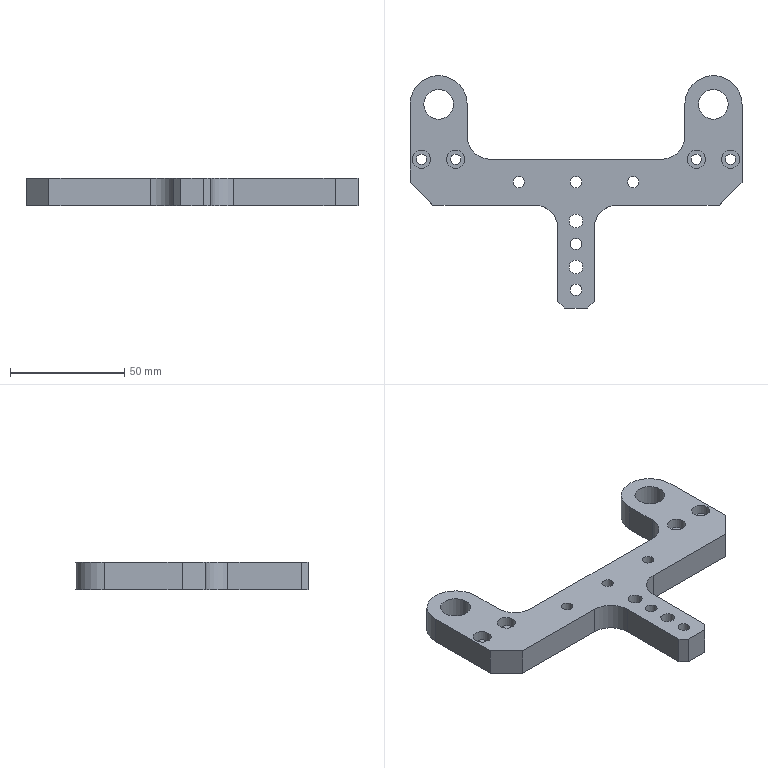Part | NX | features BREP 1 | 1 solid | 59 faces | box 145 x 101.5 x 12 mm | volume 56468 mm3 | cylinder 31 | plane 20 | cone 8 | commonest cylinder face diameters 5 x5 2.5 x4 4 x4 4.5 x4 8 x4 20 x4
STEP:
#1=CARTESIAN_POINT('',(2.5,55.,0.));
#2=VERTEX_POINT('',#1);
#3=CARTESIAN_POINT('',(0.,55.,0.));
#4=DIRECTION('',(0.,0.,1.));
#5=DIRECTION('',(1.,0.,0.));
#6=AXIS2_PLACEMENT_3D('',#3,#4,#5);
#7=CIRCLE('',#6,2.5);
#8=EDGE_CURVE('',#2,#2,#7,.T.);
#9=ORIENTED_EDGE('',*,*,#8,.T.);
#10=EDGE_LOOP('',(#9));
#11=FACE_BOUND('',#10,.T.);
#12=CARTESIAN_POINT('',(22.5,55.,0.));
#13=VERTEX_POINT('',#12);
#14=CARTESIAN_POINT('',(25.,55.,0.));
#15=DIRECTION('',(0.,0.,-1.));
#16=DIRECTION('',(-1.,0.,0.));
#17=AXIS2_PLACEMENT_3D('',#14,#15,#16);
#18=CIRCLE('',#17,2.5);
#19=EDGE_CURVE('',#13,#13,#18,.T.);
#20=ORIENTED_EDGE('',*,*,#19,.F.);
#21=EDGE_LOOP('',(#20));
#22=FACE_BOUND('',#21,.T.);
#23=CARTESIAN_POINT('',(-70.75,89.,0.));
#24=VERTEX_POINT('',#23);
#25=CARTESIAN_POINT('',(-69.5,89.,0.));
#26=DIRECTION('',(0.,0.,-1.));
#27=DIRECTION('',(-1.,0.,0.));
#28=AXIS2_PLACEMENT_3D('',#25,#26,#27);
#29=CIRCLE('',#28,1.25);
#30=EDGE_CURVE('',#24,#24,#29,.T.);
#31=ORIENTED_EDGE('',*,*,#30,.F.);
#32=EDGE_LOOP('',(#31));
#33=FACE_BOUND('',#32,.T.);
#34=CARTESIAN_POINT('',(-51.75,89.,0.));
#35=VERTEX_POINT('',#34);
#36=CARTESIAN_POINT('',(-50.5,89.,0.));
#37=DIRECTION('',(0.,0.,-1.));
#38=DIRECTION('',(-1.,0.,0.));
#39=AXIS2_PLACEMENT_3D('',#36,#37,#38);
#40=CIRCLE('',#39,1.25);
#41=EDGE_CURVE('',#35,#35,#40,.T.);
#42=ORIENTED_EDGE('',*,*,#41,.F.);
#43=EDGE_LOOP('',(#42));
#44=FACE_BOUND('',#43,.T.);
#45=CARTESIAN_POINT('',(68.25,89.,0.));
#46=VERTEX_POINT('',#45);
#47=CARTESIAN_POINT('',(69.5,89.,0.));
#48=DIRECTION('',(0.,0.,-1.));
#49=DIRECTION('',(-1.,0.,0.));
#50=AXIS2_PLACEMENT_3D('',#47,#48,#49);
#51=CIRCLE('',#50,1.25);
#52=EDGE_CURVE('',#46,#46,#51,.T.);
#53=ORIENTED_EDGE('',*,*,#52,.F.);
#54=EDGE_LOOP('',(#53));
#55=FACE_BOUND('',#54,.T.);
#56=CARTESIAN_POINT('',(49.25,89.,0.));
#57=VERTEX_POINT('',#56);
#58=CARTESIAN_POINT('',(50.5,89.,0.));
#59=DIRECTION('',(0.,0.,-1.));
#60=DIRECTION('',(-1.,0.,0.));
#61=AXIS2_PLACEMENT_3D('',#58,#59,#60);
#62=CIRCLE('',#61,1.25);
#63=EDGE_CURVE('',#57,#57,#62,.T.);
#64=ORIENTED_EDGE('',*,*,#63,.F.);
#65=EDGE_LOOP('',(#64));
#66=FACE_BOUND('',#65,.T.);
#67=CARTESIAN_POINT('',(-2.5,8.,0.));
#68=VERTEX_POINT('',#67);
#69=CARTESIAN_POINT('',(0.,8.,0.));
#70=DIRECTION('',(0.,0.,-1.));
#71=DIRECTION('',(-1.,0.,0.));
#72=AXIS2_PLACEMENT_3D('',#69,#70,#71);
#73=CIRCLE('',#72,2.5);
#74=EDGE_CURVE('',#68,#68,#73,.T.);
#75=ORIENTED_EDGE('',*,*,#74,.F.);
#76=EDGE_LOOP('',(#75));
#77=FACE_BOUND('',#76,.T.);
#78=CARTESIAN_POINT('',(-2.5,28.,0.));
#79=VERTEX_POINT('',#78);
#80=CARTESIAN_POINT('',(0.,28.,0.));
#81=DIRECTION('',(0.,0.,-1.));
#82=DIRECTION('',(-1.,0.,0.));
#83=AXIS2_PLACEMENT_3D('',#80,#81,#82);
#84=CIRCLE('',#83,2.5);
#85=EDGE_CURVE('',#79,#79,#84,.T.);
#86=ORIENTED_EDGE('',*,*,#85,.F.);
#87=EDGE_LOOP('',(#86));
#88=FACE_BOUND('',#87,.T.);
#89=CARTESIAN_POINT('',(-3.,38.,0.));
#90=VERTEX_POINT('',#89);
#91=CARTESIAN_POINT('',(0.,38.,0.));
#92=DIRECTION('',(0.,0.,-1.));
#93=DIRECTION('',(-1.,0.,0.));
#94=AXIS2_PLACEMENT_3D('',#91,#92,#93);
#95=CIRCLE('',#94,3.);
#96=EDGE_CURVE('',#90,#90,#95,.T.);
#97=ORIENTED_EDGE('',*,*,#96,.F.);
#98=EDGE_LOOP('',(#97));
#99=FACE_BOUND('',#98,.T.);
#100=CARTESIAN_POINT('',(-62.,79.5,0.));
#101=VERTEX_POINT('',#100);
#102=CARTESIAN_POINT('',(-60.,79.5,0.));
#103=DIRECTION('',(0.,0.,-1.));
#104=DIRECTION('',(-1.,0.,0.));
#105=AXIS2_PLACEMENT_3D('',#102,#103,#104);
#106=CIRCLE('',#105,2.);
#107=EDGE_CURVE('',#101,#101,#106,.T.);
#108=ORIENTED_EDGE('',*,*,#107,.F.);
#109=EDGE_LOOP('',(#108));
#110=FACE_BOUND('',#109,.T.);
#111=CARTESIAN_POINT('',(-62.,98.5,0.));
#112=VERTEX_POINT('',#111);
#113=CARTESIAN_POINT('',(-60.,98.5,0.));
#114=DIRECTION('',(0.,0.,-1.));
#115=DIRECTION('',(-1.,0.,0.));
#116=AXIS2_PLACEMENT_3D('',#113,#114,#115);
#117=CIRCLE('',#116,2.);
#118=EDGE_CURVE('',#112,#112,#117,.T.);
#119=ORIENTED_EDGE('',*,*,#118,.F.);
#120=EDGE_LOOP('',(#119));
#121=FACE_BOUND('',#120,.T.);
#122=CARTESIAN_POINT('',(58.,79.5,0.));
#123=VERTEX_POINT('',#122);
#124=CARTESIAN_POINT('',(60.,79.5,0.));
#125=DIRECTION('',(0.,0.,-1.));
#126=DIRECTION('',(-1.,0.,0.));
#127=AXIS2_PLACEMENT_3D('',#124,#125,#126);
#128=CIRCLE('',#127,2.);
#129=EDGE_CURVE('',#123,#123,#128,.T.);
#130=ORIENTED_EDGE('',*,*,#129,.F.);
#131=EDGE_LOOP('',(#130));
#132=FACE_BOUND('',#131,.T.);
#133=CARTESIAN_POINT('',(58.,98.5,0.));
#134=VERTEX_POINT('',#133);
#135=CARTESIAN_POINT('',(60.,98.5,0.));
#136=DIRECTION('',(0.,0.,-1.));
#137=DIRECTION('',(-1.,0.,0.));
#138=AXIS2_PLACEMENT_3D('',#135,#136,#137);
#139=CIRCLE('',#138,2.);
#140=EDGE_CURVE('',#134,#134,#139,.T.);
#141=ORIENTED_EDGE('',*,*,#140,.F.);
#142=EDGE_LOOP('',(#141));
#143=FACE_BOUND('',#142,.T.);
#144=CARTESIAN_POINT('',(69.75,65.,0.));
#145=VERTEX_POINT('',#144);
#146=CARTESIAN_POINT('',(67.5,65.,0.));
#147=DIRECTION('',(0.,0.,1.));
#148=DIRECTION('',(1.,0.,0.));
#149=AXIS2_PLACEMENT_3D('',#146,#147,#148);
#150=CIRCLE('',#149,2.25);
#151=EDGE_CURVE('',#145,#145,#150,.T.);
#152=ORIENTED_EDGE('',*,*,#151,.T.);
#153=EDGE_LOOP('',(#152));
#154=FACE_BOUND('',#153,.T.);
#155=CARTESIAN_POINT('',(54.75,65.,0.));
#156=VERTEX_POINT('',#155);
#157=CARTESIAN_POINT('',(52.5,65.,0.));
#158=DIRECTION('',(0.,0.,1.));
#159=DIRECTION('',(1.,0.,0.));
#160=AXIS2_PLACEMENT_3D('',#157,#158,#159);
#161=CIRCLE('',#160,2.25);
#162=EDGE_CURVE('',#156,#156,#161,.T.);
#163=ORIENTED_EDGE('',*,*,#162,.T.);
#164=EDGE_LOOP('',(#163));
#165=FACE_BOUND('',#164,.T.);
#166=CARTESIAN_POINT('',(-65.25,65.,0.));
#167=VERTEX_POINT('',#166);
#168=CARTESIAN_POINT('',(-67.5,65.,0.));
#169=DIRECTION('',(0.,0.,1.));
#170=DIRECTION('',(1.,0.,0.));
#171=AXIS2_PLACEMENT_3D('',#168,#169,#170);
#172=CIRCLE('',#171,2.25);
#173=EDGE_CURVE('',#167,#167,#172,.T.);
#174=ORIENTED_EDGE('',*,*,#173,.T.);
#175=EDGE_LOOP('',(#174));
#176=FACE_BOUND('',#175,.T.);
#177=CARTESIAN_POINT('',(-50.25,65.,0.));
#178=VERTEX_POINT('',#177);
#179=CARTESIAN_POINT('',(-52.5,65.,0.));
#180=DIRECTION('',(0.,0.,1.));
#181=DIRECTION('',(1.,0.,0.));
#182=AXIS2_PLACEMENT_3D('',#179,#180,#181);
#183=CIRCLE('',#182,2.25);
#184=EDGE_CURVE('',#178,#178,#183,.T.);
#185=ORIENTED_EDGE('',*,*,#184,.T.);
#186=EDGE_LOOP('',(#185));
#187=FACE_BOUND('',#186,.T.);
#188=CARTESIAN_POINT('',(66.5,89.,0.));
#189=VERTEX_POINT('',#188);
#190=CARTESIAN_POINT('',(60.,89.,0.));
#191=DIRECTION('',(0.,0.,1.));
#192=DIRECTION('',(1.,0.,0.));
#193=AXIS2_PLACEMENT_3D('',#190,#191,#192);
#194=CIRCLE('',#193,6.5);
#195=EDGE_CURVE('',#189,#189,#194,.T.);
#196=ORIENTED_EDGE('',*,*,#195,.T.);
#197=EDGE_LOOP('',(#196));
#198=FACE_BOUND('',#197,.T.);
#199=CARTESIAN_POINT('',(-53.5,89.,0.));
#200=VERTEX_POINT('',#199);
#201=CARTESIAN_POINT('',(-60.,89.,0.));
#202=DIRECTION('',(0.,0.,1.));
#203=DIRECTION('',(1.,0.,0.));
#204=AXIS2_PLACEMENT_3D('',#201,#202,#203);
#205=CIRCLE('',#204,6.5);
#206=EDGE_CURVE('',#200,#200,#205,.T.);
#207=ORIENTED_EDGE('',*,*,#206,.T.);
#208=EDGE_LOOP('',(#207));
#209=FACE_BOUND('',#208,.T.);
#210=CARTESIAN_POINT('',(8.,3.,0.));
#211=VERTEX_POINT('',#210);
#212=CARTESIAN_POINT('',(8.,35.,0.));
#213=VERTEX_POINT('',#212);
#214=CARTESIAN_POINT('',(8.,0.,0.));
#215=DIRECTION('',(0.,1.,0.));
#216=VECTOR('',#215,1000.);
#217=LINE('',#214,#216);
#218=EDGE_CURVE('',#211,#213,#217,.T.);
#219=ORIENTED_EDGE('',*,*,#218,.F.);
#220=CARTESIAN_POINT('',(5.,0.,0.));
#221=VERTEX_POINT('',#220);
#222=CARTESIAN_POINT('',(8.,3.,0.));
#223=DIRECTION('',(-0.7071,-0.7071,0.));
#224=VECTOR('',#223,1000.);
#225=LINE('',#222,#224);
#226=EDGE_CURVE('',#211,#221,#225,.T.);
#227=ORIENTED_EDGE('',*,*,#226,.T.);
#228=CARTESIAN_POINT('',(-5.,0.,0.));
#229=VERTEX_POINT('',#228);
#230=CARTESIAN_POINT('',(-8.,0.,0.));
#231=DIRECTION('',(1.,0.,0.));
#232=VECTOR('',#231,1000.);
#233=LINE('',#230,#232);
#234=EDGE_CURVE('',#229,#221,#233,.T.);
#235=ORIENTED_EDGE('',*,*,#234,.F.);
#236=CARTESIAN_POINT('',(-8.,3.,0.));
#237=VERTEX_POINT('',#236);
#238=CARTESIAN_POINT('',(-5.,0.,0.));
#239=DIRECTION('',(-0.7071,0.7071,0.));
#240=VECTOR('',#239,1000.);
#241=LINE('',#238,#240);
#242=EDGE_CURVE('',#229,#237,#241,.T.);
#243=ORIENTED_EDGE('',*,*,#242,.T.);
#244=CARTESIAN_POINT('',(-8.,35.,0.));
#245=VERTEX_POINT('',#244);
#246=CARTESIAN_POINT('',(-8.,45.,0.));
#247=DIRECTION('',(0.,-1.,0.));
#248=VECTOR('',#247,1000.);
#249=LINE('',#246,#248);
#250=EDGE_CURVE('',#245,#237,#249,.T.);
#251=ORIENTED_EDGE('',*,*,#250,.F.);
#252=CARTESIAN_POINT('',(-18.,45.,0.));
#253=VERTEX_POINT('',#252);
#254=CARTESIAN_POINT('',(-18.,35.,0.));
#255=DIRECTION('',(0.,0.,1.));
#256=DIRECTION('',(1.,0.,0.));
#257=AXIS2_PLACEMENT_3D('',#254,#255,#256);
#258=CIRCLE('',#257,10.);
#259=EDGE_CURVE('',#245,#253,#258,.T.);
#260=ORIENTED_EDGE('',*,*,#259,.T.);
#261=CARTESIAN_POINT('',(-62.5,45.,0.));
#262=VERTEX_POINT('',#261);
#263=CARTESIAN_POINT('',(-72.5,45.,0.));
#264=DIRECTION('',(1.,0.,0.));
#265=VECTOR('',#264,1000.);
#266=LINE('',#263,#265);
#267=EDGE_CURVE('',#262,#253,#266,.T.);
#268=ORIENTED_EDGE('',*,*,#267,.F.);
#269=CARTESIAN_POINT('',(-72.5,55.,0.));
#270=VERTEX_POINT('',#269);
#271=CARTESIAN_POINT('',(-62.5,45.,0.));
#272=DIRECTION('',(-0.7071,0.7071,0.));
#273=VECTOR('',#272,1000.);
#274=LINE('',#271,#273);
#275=EDGE_CURVE('',#262,#270,#274,.T.);
#276=ORIENTED_EDGE('',*,*,#275,.T.);
#277=CARTESIAN_POINT('',(-72.5,89.,0.));
#278=VERTEX_POINT('',#277);
#279=CARTESIAN_POINT('',(-72.5,89.,0.));
#280=DIRECTION('',(0.,-1.,0.));
#281=VECTOR('',#280,1000.);
#282=LINE('',#279,#281);
#283=EDGE_CURVE('',#278,#270,#282,.T.);
#284=ORIENTED_EDGE('',*,*,#283,.F.);
#285=CARTESIAN_POINT('',(-47.5,89.,0.));
#286=VERTEX_POINT('',#285);
#287=CARTESIAN_POINT('',(-60.,89.,0.));
#288=DIRECTION('',(0.,0.,1.));
#289=DIRECTION('',(1.,0.,0.));
#290=AXIS2_PLACEMENT_3D('',#287,#288,#289);
#291=CIRCLE('',#290,12.5);
#292=EDGE_CURVE('',#286,#278,#291,.T.);
#293=ORIENTED_EDGE('',*,*,#292,.F.);
#294=CARTESIAN_POINT('',(-47.5,75.,0.));
#295=VERTEX_POINT('',#294);
#296=CARTESIAN_POINT('',(-47.5,65.,0.));
#297=DIRECTION('',(0.,1.,0.));
#298=VECTOR('',#297,1000.);
#299=LINE('',#296,#298);
#300=EDGE_CURVE('',#295,#286,#299,.T.);
#301=ORIENTED_EDGE('',*,*,#300,.F.);
#302=CARTESIAN_POINT('',(-37.5,65.,0.));
#303=VERTEX_POINT('',#302);
#304=CARTESIAN_POINT('',(-37.5,75.,0.));
#305=DIRECTION('',(0.,0.,1.));
#306=DIRECTION('',(1.,0.,0.));
#307=AXIS2_PLACEMENT_3D('',#304,#305,#306);
#308=CIRCLE('',#307,10.);
#309=EDGE_CURVE('',#295,#303,#308,.T.);
#310=ORIENTED_EDGE('',*,*,#309,.T.);
#311=CARTESIAN_POINT('',(37.5,65.,0.));
#312=VERTEX_POINT('',#311);
#313=CARTESIAN_POINT('',(47.5,65.,0.));
#314=DIRECTION('',(-1.,0.,0.));
#315=VECTOR('',#314,1000.);
#316=LINE('',#313,#315);
#317=EDGE_CURVE('',#312,#303,#316,.T.);
#318=ORIENTED_EDGE('',*,*,#317,.F.);
#319=CARTESIAN_POINT('',(47.5,75.,0.));
#320=VERTEX_POINT('',#319);
#321=CARTESIAN_POINT('',(37.5,75.,0.));
#322=DIRECTION('',(0.,0.,1.));
#323=DIRECTION('',(1.,0.,0.));
#324=AXIS2_PLACEMENT_3D('',#321,#322,#323);
#325=CIRCLE('',#324,10.);
#326=EDGE_CURVE('',#312,#320,#325,.T.);
#327=ORIENTED_EDGE('',*,*,#326,.T.);
#328=CARTESIAN_POINT('',(47.5,89.,0.));
#329=VERTEX_POINT('',#328);
#330=CARTESIAN_POINT('',(47.5,89.,0.));
#331=DIRECTION('',(0.,-1.,0.));
#332=VECTOR('',#331,1000.);
#333=LINE('',#330,#332);
#334=EDGE_CURVE('',#329,#320,#333,.T.);
#335=ORIENTED_EDGE('',*,*,#334,.F.);
#336=CARTESIAN_POINT('',(72.5,89.,0.));
#337=VERTEX_POINT('',#336);
#338=CARTESIAN_POINT('',(60.,89.,0.));
#339=DIRECTION('',(0.,0.,1.));
#340=DIRECTION('',(1.,0.,0.));
#341=AXIS2_PLACEMENT_3D('',#338,#339,#340);
#342=CIRCLE('',#341,12.5);
#343=EDGE_CURVE('',#337,#329,#342,.T.);
#344=ORIENTED_EDGE('',*,*,#343,.F.);
#345=CARTESIAN_POINT('',(72.5,55.,0.));
#346=VERTEX_POINT('',#345);
#347=CARTESIAN_POINT('',(72.5,45.,0.));
#348=DIRECTION('',(0.,1.,0.));
#349=VECTOR('',#348,1000.);
#350=LINE('',#347,#349);
#351=EDGE_CURVE('',#346,#337,#350,.T.);
#352=ORIENTED_EDGE('',*,*,#351,.F.);
#353=CARTESIAN_POINT('',(62.5,45.,0.));
#354=VERTEX_POINT('',#353);
#355=CARTESIAN_POINT('',(72.5,55.,0.));
#356=DIRECTION('',(-0.7071,-0.7071,0.));
#357=VECTOR('',#356,1000.);
#358=LINE('',#355,#357);
#359=EDGE_CURVE('',#346,#354,#358,.T.);
#360=ORIENTED_EDGE('',*,*,#359,.T.);
#361=CARTESIAN_POINT('',(18.,45.,0.));
#362=VERTEX_POINT('',#361);
#363=CARTESIAN_POINT('',(8.,45.,0.));
#364=DIRECTION('',(1.,0.,0.));
#365=VECTOR('',#364,1000.);
#366=LINE('',#363,#365);
#367=EDGE_CURVE('',#362,#354,#366,.T.);
#368=ORIENTED_EDGE('',*,*,#367,.F.);
#369=CARTESIAN_POINT('',(18.,35.,0.));
#370=DIRECTION('',(0.,0.,1.));
#371=DIRECTION('',(1.,0.,0.));
#372=AXIS2_PLACEMENT_3D('',#369,#370,#371);
#373=CIRCLE('',#372,10.);
#374=EDGE_CURVE('',#362,#213,#373,.T.);
#375=ORIENTED_EDGE('',*,*,#374,.T.);
#376=EDGE_LOOP('',(#219,#227,#235,#243,#251,#260,#268,#276,#284,#293,#301,#310,#318,#327,#335,#344,#352,#360,#368,#375));
#377=FACE_BOUND('',#376,.T.);
#378=CARTESIAN_POINT('',(-3.,18.,0.));
#379=VERTEX_POINT('',#378);
#380=CARTESIAN_POINT('',(0.,18.,0.));
#381=DIRECTION('',(0.,0.,-1.));
#382=DIRECTION('',(-1.,0.,0.));
#383=AXIS2_PLACEMENT_3D('',#380,#381,#382);
#384=CIRCLE('',#383,3.);
#385=EDGE_CURVE('',#379,#379,#384,.T.);
#386=ORIENTED_EDGE('',*,*,#385,.F.);
#387=EDGE_LOOP('',(#386));
#388=FACE_BOUND('',#387,.T.);
#389=CARTESIAN_POINT('',(-27.5,55.,0.));
#390=VERTEX_POINT('',#389);
#391=CARTESIAN_POINT('',(-25.,55.,0.));
#392=DIRECTION('',(0.,0.,-1.));
#393=DIRECTION('',(-1.,0.,0.));
#394=AXIS2_PLACEMENT_3D('',#391,#392,#393);
#395=CIRCLE('',#394,2.5);
#396=EDGE_CURVE('',#390,#390,#395,.T.);
#397=ORIENTED_EDGE('',*,*,#396,.F.);
#398=EDGE_LOOP('',(#397));
#399=FACE_BOUND('',#398,.T.);
#400=CARTESIAN_POINT('',(60.,89.,0.));
#401=DIRECTION('',(0.,0.,1.));
#402=DIRECTION('',(-1.,0.,0.));
#403=AXIS2_PLACEMENT_3D('',#400,#401,#402);
#404=PLANE('',#403);
#405=ADVANCED_FACE('',(#11,#22,#33,#44,#55,#66,#77,#88,#99,#110,#121,#132,#143,#154,#165,#176,#187,#198,#209,#377,#388,#399),#404,.F.);
#406=CARTESIAN_POINT('',(2.5,55.,12.));
#407=VERTEX_POINT('',#406);
#408=CARTESIAN_POINT('',(0.,55.,12.));
#409=DIRECTION('',(0.,0.,1.));
#410=DIRECTION('',(1.,0.,0.));
#411=AXIS2_PLACEMENT_3D('',#408,#409,#410);
#412=CIRCLE('',#411,2.5);
#413=EDGE_CURVE('',#407,#407,#412,.T.);
#414=ORIENTED_EDGE('',*,*,#413,.F.);
#415=EDGE_LOOP('',(#414));
#416=FACE_BOUND('',#415,.T.);
#417=CARTESIAN_POINT('',(-27.5,55.,12.));
#418=VERTEX_POINT('',#417);
#419=CARTESIAN_POINT('',(-25.,55.,12.));
#420=DIRECTION('',(0.,0.,-1.));
#421=DIRECTION('',(-1.,0.,0.));
#422=AXIS2_PLACEMENT_3D('',#419,#420,#421);
#423=CIRCLE('',#422,2.5);
#424=EDGE_CURVE('',#418,#418,#423,.T.);
#425=ORIENTED_EDGE('',*,*,#424,.T.);
#426=EDGE_LOOP('',(#425));
#427=FACE_BOUND('',#426,.T.);
#428=CARTESIAN_POINT('',(22.5,55.,12.));
#429=VERTEX_POINT('',#428);
#430=CARTESIAN_POINT('',(25.,55.,12.));
#431=DIRECTION('',(0.,0.,-1.));
#432=DIRECTION('',(-1.,0.,0.));
#433=AXIS2_PLACEMENT_3D('',#430,#431,#432);
#434=CIRCLE('',#433,2.5);
#435=EDGE_CURVE('',#429,#429,#434,.T.);
#436=ORIENTED_EDGE('',*,*,#435,.T.);
#437=EDGE_LOOP('',(#436));
#438=FACE_BOUND('',#437,.T.);
#439=CARTESIAN_POINT('',(-2.5,8.,12.));
#440=VERTEX_POINT('',#439);
#441=CARTESIAN_POINT('',(0.,8.,12.));
#442=DIRECTION('',(0.,0.,-1.));
#443=DIRECTION('',(-1.,0.,0.));
#444=AXIS2_PLACEMENT_3D('',#441,#442,#443);
#445=CIRCLE('',#444,2.5);
#446=EDGE_CURVE('',#440,#440,#445,.T.);
#447=ORIENTED_EDGE('',*,*,#446,.T.);
#448=EDGE_LOOP('',(#447));
#449=FACE_BOUND('',#448,.T.);
#450=CARTESIAN_POINT('',(-5.,0.,12.));
#451=VERTEX_POINT('',#450);
#452=CARTESIAN_POINT('',(5.,0.,12.));
#453=VERTEX_POINT('',#452);
#454=CARTESIAN_POINT('',(-8.,0.,12.));
#455=DIRECTION('',(1.,0.,0.));
#456=VECTOR('',#455,1000.);
#457=LINE('',#454,#456);
#458=EDGE_CURVE('',#451,#453,#457,.T.);
#459=ORIENTED_EDGE('',*,*,#458,.T.);
#460=CARTESIAN_POINT('',(8.,3.,12.));
#461=VERTEX_POINT('',#460);
#462=CARTESIAN_POINT('',(77.,72.,12.));
#463=DIRECTION('',(0.7071,0.7071,0.));
#464=VECTOR('',#463,1000.);
#465=LINE('',#462,#464);
#466=EDGE_CURVE('',#453,#461,#465,.T.);
#467=ORIENTED_EDGE('',*,*,#466,.T.);
#468=CARTESIAN_POINT('',(8.,35.,12.));
#469=VERTEX_POINT('',#468);
#470=CARTESIAN_POINT('',(8.,0.,12.));
#471=DIRECTION('',(0.,1.,0.));
#472=VECTOR('',#471,1000.);
#473=LINE('',#470,#472);
#474=EDGE_CURVE('',#461,#469,#473,.T.);
#475=ORIENTED_EDGE('',*,*,#474,.T.);
#476=CARTESIAN_POINT('',(18.,45.,12.));
#477=VERTEX_POINT('',#476);
#478=CARTESIAN_POINT('',(18.,35.,12.));
#479=DIRECTION('',(0.,0.,-1.));
#480=DIRECTION('',(1.,0.,0.));
#481=AXIS2_PLACEMENT_3D('',#478,#479,#480);
#482=CIRCLE('',#481,10.);
#483=EDGE_CURVE('',#469,#477,#482,.T.);
#484=ORIENTED_EDGE('',*,*,#483,.T.);
#485=CARTESIAN_POINT('',(62.5,45.,12.));
#486=VERTEX_POINT('',#485);
#487=CARTESIAN_POINT('',(8.,45.,12.));
#488=DIRECTION('',(1.,0.,0.));
#489=VECTOR('',#488,1000.);
#490=LINE('',#487,#489);
#491=EDGE_CURVE('',#477,#486,#490,.T.);
#492=ORIENTED_EDGE('',*,*,#491,.T.);
#493=CARTESIAN_POINT('',(72.5,55.,12.));
#494=VERTEX_POINT('',#493);
#495=CARTESIAN_POINT('',(83.25,65.75,12.));
#496=DIRECTION('',(0.7071,0.7071,0.));
#497=VECTOR('',#496,1000.);
#498=LINE('',#495,#497);
#499=EDGE_CURVE('',#486,#494,#498,.T.);
#500=ORIENTED_EDGE('',*,*,#499,.T.);
#501=CARTESIAN_POINT('',(72.5,89.,12.));
#502=VERTEX_POINT('',#501);
#503=CARTESIAN_POINT('',(72.5,45.,12.));
#504=DIRECTION('',(0.,1.,0.));
#505=VECTOR('',#504,1000.);
#506=LINE('',#503,#505);
#507=EDGE_CURVE('',#494,#502,#506,.T.);
#508=ORIENTED_EDGE('',*,*,#507,.T.);
#509=CARTESIAN_POINT('',(47.5,89.,12.));
#510=VERTEX_POINT('',#509);
#511=CARTESIAN_POINT('',(60.,89.,12.));
#512=DIRECTION('',(0.,0.,1.));
#513=DIRECTION('',(1.,0.,0.));
#514=AXIS2_PLACEMENT_3D('',#511,#512,#513);
#515=CIRCLE('',#514,12.5);
#516=EDGE_CURVE('',#502,#510,#515,.T.);
#517=ORIENTED_EDGE('',*,*,#516,.T.);
#518=CARTESIAN_POINT('',(47.5,75.,12.));
#519=VERTEX_POINT('',#518);
#520=CARTESIAN_POINT('',(47.5,89.,12.));
#521=DIRECTION('',(0.,-1.,0.));
#522=VECTOR('',#521,1000.);
#523=LINE('',#520,#522);
#524=EDGE_CURVE('',#510,#519,#523,.T.);
#525=ORIENTED_EDGE('',*,*,#524,.T.);
#526=CARTESIAN_POINT('',(37.5,65.,12.));
#527=VERTEX_POINT('',#526);
#528=CARTESIAN_POINT('',(37.5,75.,12.));
#529=DIRECTION('',(0.,0.,-1.));
#530=DIRECTION('',(1.,0.,0.));
#531=AXIS2_PLACEMENT_3D('',#528,#529,#530);
#532=CIRCLE('',#531,10.);
#533=EDGE_CURVE('',#519,#527,#532,.T.);
#534=ORIENTED_EDGE('',*,*,#533,.T.);
#535=CARTESIAN_POINT('',(-37.5,65.,12.));
#536=VERTEX_POINT('',#535);
#537=CARTESIAN_POINT('',(47.5,65.,12.));
#538=DIRECTION('',(-1.,0.,0.));
#539=VECTOR('',#538,1000.);
#540=LINE('',#537,#539);
#541=EDGE_CURVE('',#527,#536,#540,.T.);
#542=ORIENTED_EDGE('',*,*,#541,.T.);
#543=CARTESIAN_POINT('',(-47.5,75.,12.));
#544=VERTEX_POINT('',#543);
#545=CARTESIAN_POINT('',(-37.5,75.,12.));
#546=DIRECTION('',(0.,0.,-1.));
#547=DIRECTION('',(1.,0.,0.));
#548=AXIS2_PLACEMENT_3D('',#545,#546,#547);
#549=CIRCLE('',#548,10.);
#550=EDGE_CURVE('',#536,#544,#549,.T.);
#551=ORIENTED_EDGE('',*,*,#550,.T.);
#552=CARTESIAN_POINT('',(-47.5,89.,12.));
#553=VERTEX_POINT('',#552);
#554=CARTESIAN_POINT('',(-47.5,65.,12.));
#555=DIRECTION('',(0.,1.,0.));
#556=VECTOR('',#555,1000.);
#557=LINE('',#554,#556);
#558=EDGE_CURVE('',#544,#553,#557,.T.);
#559=ORIENTED_EDGE('',*,*,#558,.T.);
#560=CARTESIAN_POINT('',(-72.5,89.,12.));
#561=VERTEX_POINT('',#560);
#562=CARTESIAN_POINT('',(-60.,89.,12.));
#563=DIRECTION('',(0.,0.,1.));
#564=DIRECTION('',(1.,0.,0.));
#565=AXIS2_PLACEMENT_3D('',#562,#563,#564);
#566=CIRCLE('',#565,12.5);
#567=EDGE_CURVE('',#553,#561,#566,.T.);
#568=ORIENTED_EDGE('',*,*,#567,.T.);
#569=CARTESIAN_POINT('',(-72.5,55.,12.));
#570=VERTEX_POINT('',#569);
#571=CARTESIAN_POINT('',(-72.5,89.,12.));
#572=DIRECTION('',(0.,-1.,0.));
#573=VECTOR('',#572,1000.);
#574=LINE('',#571,#573);
#575=EDGE_CURVE('',#561,#570,#574,.T.);
#576=ORIENTED_EDGE('',*,*,#575,.T.);
#577=CARTESIAN_POINT('',(-62.5,45.,12.));
#578=VERTEX_POINT('',#577);
#579=CARTESIAN_POINT('',(-23.25,5.75,12.));
#580=DIRECTION('',(0.7071,-0.7071,0.));
#581=VECTOR('',#580,1000.);
#582=LINE('',#579,#581);
#583=EDGE_CURVE('',#570,#578,#582,.T.);
#584=ORIENTED_EDGE('',*,*,#583,.T.);
#585=CARTESIAN_POINT('',(-18.,45.,12.));
#586=VERTEX_POINT('',#585);
#587=CARTESIAN_POINT('',(-72.5,45.,12.));
#588=DIRECTION('',(1.,0.,0.));
#589=VECTOR('',#588,1000.);
#590=LINE('',#587,#589);
#591=EDGE_CURVE('',#578,#586,#590,.T.);
#592=ORIENTED_EDGE('',*,*,#591,.T.);
#593=CARTESIAN_POINT('',(-8.,35.,12.));
#594=VERTEX_POINT('',#593);
#595=CARTESIAN_POINT('',(-18.,35.,12.));
#596=DIRECTION('',(0.,0.,-1.));
#597=DIRECTION('',(1.,0.,0.));
#598=AXIS2_PLACEMENT_3D('',#595,#596,#597);
#599=CIRCLE('',#598,10.);
#600=EDGE_CURVE('',#586,#594,#599,.T.);
#601=ORIENTED_EDGE('',*,*,#600,.T.);
#602=CARTESIAN_POINT('',(-8.,3.,12.));
#603=VERTEX_POINT('',#602);
#604=CARTESIAN_POINT('',(-8.,45.,12.));
#605=DIRECTION('',(0.,-1.,0.));
#606=VECTOR('',#605,1000.);
#607=LINE('',#604,#606);
#608=EDGE_CURVE('',#594,#603,#607,.T.);
#609=ORIENTED_EDGE('',*,*,#608,.T.);
#610=CARTESIAN_POINT('',(-17.,12.,12.));
#611=DIRECTION('',(0.7071,-0.7071,0.));
#612=VECTOR('',#611,1000.);
#613=LINE('',#610,#612);
#614=EDGE_CURVE('',#603,#451,#613,.T.);
#615=ORIENTED_EDGE('',*,*,#614,.T.);
#616=EDGE_LOOP('',(#459,#467,#475,#484,#492,#500,#508,#517,#525,#534,#542,#551,#559,#568,#576,#584,#592,#601,#609,#615));
#617=FACE_BOUND('',#616,.T.);
#618=CARTESIAN_POINT('',(-53.5,89.,12.));
#619=VERTEX_POINT('',#618);
#620=CARTESIAN_POINT('',(-60.,89.,12.));
#621=DIRECTION('',(0.,0.,1.));
#622=DIRECTION('',(1.,0.,0.));
#623=AXIS2_PLACEMENT_3D('',#620,#621,#622);
#624=CIRCLE('',#623,6.5);
#625=EDGE_CURVE('',#619,#619,#624,.T.);
#626=ORIENTED_EDGE('',*,*,#625,.F.);
#627=EDGE_LOOP('',(#626));
#628=FACE_BOUND('',#627,.T.);
#629=CARTESIAN_POINT('',(66.5,89.,12.));
#630=VERTEX_POINT('',#629);
#631=CARTESIAN_POINT('',(60.,89.,12.));
#632=DIRECTION('',(0.,0.,1.));
#633=DIRECTION('',(1.,0.,0.));
#634=AXIS2_PLACEMENT_3D('',#631,#632,#633);
#635=CIRCLE('',#634,6.5);
#636=EDGE_CURVE('',#630,#630,#635,.T.);
#637=ORIENTED_EDGE('',*,*,#636,.F.);
#638=EDGE_LOOP('',(#637));
#639=FACE_BOUND('',#638,.T.);
#640=CARTESIAN_POINT('',(-48.5,65.,12.));
#641=VERTEX_POINT('',#640);
#642=CARTESIAN_POINT('',(-52.5,65.,12.));
#643=DIRECTION('',(0.,0.,1.));
#644=DIRECTION('',(1.,0.,0.));
#645=AXIS2_PLACEMENT_3D('',#642,#643,#644);
#646=CIRCLE('',#645,4.);
#647=EDGE_CURVE('',#641,#641,#646,.T.);
#648=ORIENTED_EDGE('',*,*,#647,.F.);
#649=EDGE_LOOP('',(#648));
#650=FACE_BOUND('',#649,.T.);
#651=CARTESIAN_POINT('',(-63.5,65.,12.));
#652=VERTEX_POINT('',#651);
#653=CARTESIAN_POINT('',(-67.5,65.,12.));
#654=DIRECTION('',(0.,0.,1.));
#655=DIRECTION('',(1.,0.,0.));
#656=AXIS2_PLACEMENT_3D('',#653,#654,#655);
#657=CIRCLE('',#656,4.);
#658=EDGE_CURVE('',#652,#652,#657,.T.);
#659=ORIENTED_EDGE('',*,*,#658,.F.);
#660=EDGE_LOOP('',(#659));
#661=FACE_BOUND('',#660,.T.);
#662=CARTESIAN_POINT('',(56.5,65.,12.));
#663=VERTEX_POINT('',#662);
#664=CARTESIAN_POINT('',(52.5,65.,12.));
#665=DIRECTION('',(0.,0.,1.));
#666=DIRECTION('',(1.,0.,0.));
#667=AXIS2_PLACEMENT_3D('',#664,#665,#666);
#668=CIRCLE('',#667,4.);
#669=EDGE_CURVE('',#663,#663,#668,.T.);
#670=ORIENTED_EDGE('',*,*,#669,.F.);
#671=EDGE_LOOP('',(#670));
#672=FACE_BOUND('',#671,.T.);
#673=CARTESIAN_POINT('',(71.5,65.,12.));
#674=VERTEX_POINT('',#673);
#675=CARTESIAN_POINT('',(67.5,65.,12.));
#676=DIRECTION('',(0.,0.,1.));
#677=DIRECTION('',(1.,0.,0.));
#678=AXIS2_PLACEMENT_3D('',#675,#676,#677);
#679=CIRCLE('',#678,4.);
#680=EDGE_CURVE('',#674,#674,#679,.T.);
#681=ORIENTED_EDGE('',*,*,#680,.F.);
#682=EDGE_LOOP('',(#681));
#683=FACE_BOUND('',#682,.T.);
#684=CARTESIAN_POINT('',(-3.,18.,12.));
#685=VERTEX_POINT('',#684);
#686=CARTESIAN_POINT('',(0.,18.,12.));
#687=DIRECTION('',(0.,0.,-1.));
#688=DIRECTION('',(-1.,0.,0.));
#689=AXIS2_PLACEMENT_3D('',#686,#687,#688);
#690=CIRCLE('',#689,3.);
#691=EDGE_CURVE('',#685,#685,#690,.T.);
#692=ORIENTED_EDGE('',*,*,#691,.T.);
#693=EDGE_LOOP('',(#692));
#694=FACE_BOUND('',#693,.T.);
#695=CARTESIAN_POINT('',(-3.,38.,12.));
#696=VERTEX_POINT('',#695);
#697=CARTESIAN_POINT('',(0.,38.,12.));
#698=DIRECTION('',(0.,0.,-1.));
#699=DIRECTION('',(-1.,0.,0.));
#700=AXIS2_PLACEMENT_3D('',#697,#698,#699);
#701=CIRCLE('',#700,3.);
#702=EDGE_CURVE('',#696,#696,#701,.T.);
#703=ORIENTED_EDGE('',*,*,#702,.T.);
#704=EDGE_LOOP('',(#703));
#705=FACE_BOUND('',#704,.T.);
#706=CARTESIAN_POINT('',(-2.5,28.,12.));
#707=VERTEX_POINT('',#706);
#708=CARTESIAN_POINT('',(0.,28.,12.));
#709=DIRECTION('',(0.,0.,-1.));
#710=DIRECTION('',(-1.,0.,0.));
#711=AXIS2_PLACEMENT_3D('',#708,#709,#710);
#712=CIRCLE('',#711,2.5);
#713=EDGE_CURVE('',#707,#707,#712,.T.);
#714=ORIENTED_EDGE('',*,*,#713,.T.);
#715=EDGE_LOOP('',(#714));
#716=FACE_BOUND('',#715,.T.);
#717=CARTESIAN_POINT('',(60.,89.,12.));
#718=DIRECTION('',(0.,0.,1.));
#719=DIRECTION('',(-1.,0.,0.));
#720=AXIS2_PLACEMENT_3D('',#717,#718,#719);
#721=PLANE('',#720);
#722=ADVANCED_FACE('',(#416,#427,#438,#449,#617,#628,#639,#650,#661,#672,#683,#694,#705,#716),#721,.T.);
#723=ORIENTED_EDGE('',*,*,#250,.T.);
#724=CARTESIAN_POINT('',(-8.,3.,12.));
#725=DIRECTION('',(0.,0.,1.));
#726=VECTOR('',#725,1000.);
#727=LINE('',#724,#726);
#728=EDGE_CURVE('',#237,#603,#727,.T.);
#729=ORIENTED_EDGE('',*,*,#728,.T.);
#730=ORIENTED_EDGE('',*,*,#608,.F.);
#731=CARTESIAN_POINT('',(-8.,35.,0.));
#732=DIRECTION('',(0.,0.,-1.));
#733=VECTOR('',#732,1000.);
#734=LINE('',#731,#733);
#735=EDGE_CURVE('',#594,#245,#734,.T.);
#736=ORIENTED_EDGE('',*,*,#735,.T.);
#737=EDGE_LOOP('',(#723,#729,#730,#736));
#738=FACE_BOUND('',#737,.T.);
#739=CARTESIAN_POINT('',(-8.,45.,12.));
#740=DIRECTION('',(1.,0.,0.));
#741=DIRECTION('',(0.,-1.,0.));
#742=AXIS2_PLACEMENT_3D('',#739,#740,#741);
#743=PLANE('',#742);
#744=ADVANCED_FACE('',(#738),#743,.F.);
#745=ORIENTED_EDGE('',*,*,#234,.T.);
#746=CARTESIAN_POINT('',(5.,0.,12.));
#747=DIRECTION('',(0.,0.,1.));
#748=VECTOR('',#747,1000.);
#749=LINE('',#746,#748);
#750=EDGE_CURVE('',#221,#453,#749,.T.);
#751=ORIENTED_EDGE('',*,*,#750,.T.);
#752=ORIENTED_EDGE('',*,*,#458,.F.);
#753=CARTESIAN_POINT('',(-5.,0.,12.));
#754=DIRECTION('',(0.,0.,-1.));
#755=VECTOR('',#754,1000.);
#756=LINE('',#753,#755);
#757=EDGE_CURVE('',#451,#229,#756,.T.);
#758=ORIENTED_EDGE('',*,*,#757,.T.);
#759=EDGE_LOOP('',(#745,#751,#752,#758));
#760=FACE_BOUND('',#759,.T.);
#761=CARTESIAN_POINT('',(-8.,0.,12.));
#762=DIRECTION('',(0.,1.,0.));
#763=DIRECTION('',(0.,0.,-1.));
#764=AXIS2_PLACEMENT_3D('',#761,#762,#763);
#765=PLANE('',#764);
#766=ADVANCED_FACE('',(#760),#765,.F.);
#767=ORIENTED_EDGE('',*,*,#474,.F.);
#768=CARTESIAN_POINT('',(8.,3.,12.));
#769=DIRECTION('',(0.,0.,-1.));
#770=VECTOR('',#769,1000.);
#771=LINE('',#768,#770);
#772=EDGE_CURVE('',#461,#211,#771,.T.);
#773=ORIENTED_EDGE('',*,*,#772,.T.);
#774=ORIENTED_EDGE('',*,*,#218,.T.);
#775=CARTESIAN_POINT('',(8.,35.,12.));
#776=DIRECTION('',(0.,0.,1.));
#777=VECTOR('',#776,1000.);
#778=LINE('',#775,#777);
#779=EDGE_CURVE('',#213,#469,#778,.T.);
#780=ORIENTED_EDGE('',*,*,#779,.T.);
#781=EDGE_LOOP('',(#767,#773,#774,#780));
#782=FACE_BOUND('',#781,.T.);
#783=CARTESIAN_POINT('',(8.,0.,12.));
#784=DIRECTION('',(-1.,0.,0.));
#785=DIRECTION('',(0.,1.,0.));
#786=AXIS2_PLACEMENT_3D('',#783,#784,#785);
#787=PLANE('',#786);
#788=ADVANCED_FACE('',(#782),#787,.F.);
#789=ORIENTED_EDGE('',*,*,#367,.T.);
#790=CARTESIAN_POINT('',(62.5,45.,12.));
#791=DIRECTION('',(0.,0.,1.));
#792=VECTOR('',#791,1000.);
#793=LINE('',#790,#792);
#794=EDGE_CURVE('',#354,#486,#793,.T.);
#795=ORIENTED_EDGE('',*,*,#794,.T.);
#796=ORIENTED_EDGE('',*,*,#491,.F.);
#797=CARTESIAN_POINT('',(18.,45.,0.));
#798=DIRECTION('',(0.,0.,-1.));
#799=VECTOR('',#798,1000.);
#800=LINE('',#797,#799);
#801=EDGE_CURVE('',#477,#362,#800,.T.);
#802=ORIENTED_EDGE('',*,*,#801,.T.);
#803=EDGE_LOOP('',(#789,#795,#796,#802));
#804=FACE_BOUND('',#803,.T.);
#805=CARTESIAN_POINT('',(8.,45.,12.));
#806=DIRECTION('',(0.,1.,0.));
#807=DIRECTION('',(0.,0.,-1.));
#808=AXIS2_PLACEMENT_3D('',#805,#806,#807);
#809=PLANE('',#808);
#810=ADVANCED_FACE('',(#804),#809,.F.);
#811=ORIENTED_EDGE('',*,*,#507,.F.);
#812=CARTESIAN_POINT('',(72.5,55.,12.));
#813=DIRECTION('',(0.,0.,-1.));
#814=VECTOR('',#813,1000.);
#815=LINE('',#812,#814);
#816=EDGE_CURVE('',#494,#346,#815,.T.);
#817=ORIENTED_EDGE('',*,*,#816,.T.);
#818=ORIENTED_EDGE('',*,*,#351,.T.);
#819=CARTESIAN_POINT('',(72.5,89.,12.));
#820=DIRECTION('',(0.,0.,-1.));
#821=VECTOR('',#820,1000.);
#822=LINE('',#819,#821);
#823=EDGE_CURVE('',#502,#337,#822,.T.);
#824=ORIENTED_EDGE('',*,*,#823,.F.);
#825=EDGE_LOOP('',(#811,#817,#818,#824));
#826=FACE_BOUND('',#825,.T.);
#827=CARTESIAN_POINT('',(72.5,45.,12.));
#828=DIRECTION('',(-1.,0.,0.));
#829=DIRECTION('',(0.,0.,-1.));
#830=AXIS2_PLACEMENT_3D('',#827,#828,#829);
#831=PLANE('',#830);
#832=ADVANCED_FACE('',(#826),#831,.F.);
#833=ORIENTED_EDGE('',*,*,#343,.T.);
#834=CARTESIAN_POINT('',(47.5,89.,12.));
#835=DIRECTION('',(0.,0.,-1.));
#836=VECTOR('',#835,1000.);
#837=LINE('',#834,#836);
#838=EDGE_CURVE('',#510,#329,#837,.T.);
#839=ORIENTED_EDGE('',*,*,#838,.F.);
#840=ORIENTED_EDGE('',*,*,#516,.F.);
#841=ORIENTED_EDGE('',*,*,#823,.T.);
#842=EDGE_LOOP('',(#833,#839,#840,#841));
#843=FACE_BOUND('',#842,.T.);
#844=CARTESIAN_POINT('',(60.,89.,12.));
#845=DIRECTION('',(0.,0.,-1.));
#846=DIRECTION('',(1.,0.,0.));
#847=AXIS2_PLACEMENT_3D('',#844,#845,#846);
#848=CYLINDRICAL_SURFACE('',#847,12.5);
#849=ADVANCED_FACE('',(#843),#848,.T.);
#850=ORIENTED_EDGE('',*,*,#334,.T.);
#851=CARTESIAN_POINT('',(47.5,75.,12.));
#852=DIRECTION('',(0.,0.,1.));
#853=VECTOR('',#852,1000.);
#854=LINE('',#851,#853);
#855=EDGE_CURVE('',#320,#519,#854,.T.);
#856=ORIENTED_EDGE('',*,*,#855,.T.);
#857=ORIENTED_EDGE('',*,*,#524,.F.);
#858=ORIENTED_EDGE('',*,*,#838,.T.);
#859=EDGE_LOOP('',(#850,#856,#857,#858));
#860=FACE_BOUND('',#859,.T.);
#861=CARTESIAN_POINT('',(47.5,89.,12.));
#862=DIRECTION('',(1.,0.,0.));
#863=DIRECTION('',(0.,0.,1.));
#864=AXIS2_PLACEMENT_3D('',#861,#862,#863);
#865=PLANE('',#864);
#866=ADVANCED_FACE('',(#860),#865,.F.);
#867=ORIENTED_EDGE('',*,*,#317,.T.);
#868=CARTESIAN_POINT('',(-37.5,65.,12.));
#869=DIRECTION('',(0.,0.,1.));
#870=VECTOR('',#869,1000.);
#871=LINE('',#868,#870);
#872=EDGE_CURVE('',#303,#536,#871,.T.);
#873=ORIENTED_EDGE('',*,*,#872,.T.);
#874=ORIENTED_EDGE('',*,*,#541,.F.);
#875=CARTESIAN_POINT('',(37.5,65.,0.));
#876=DIRECTION('',(0.,0.,-1.));
#877=VECTOR('',#876,1000.);
#878=LINE('',#875,#877);
#879=EDGE_CURVE('',#527,#312,#878,.T.);
#880=ORIENTED_EDGE('',*,*,#879,.T.);
#881=EDGE_LOOP('',(#867,#873,#874,#880));
#882=FACE_BOUND('',#881,.T.);
#883=CARTESIAN_POINT('',(47.5,65.,12.));
#884=DIRECTION('',(0.,-1.,0.));
#885=DIRECTION('',(0.,0.,1.));
#886=AXIS2_PLACEMENT_3D('',#883,#884,#885);
#887=PLANE('',#886);
#888=ADVANCED_FACE('',(#882),#887,.F.);
#889=ORIENTED_EDGE('',*,*,#558,.F.);
#890=CARTESIAN_POINT('',(-47.5,75.,0.));
#891=DIRECTION('',(0.,0.,-1.));
#892=VECTOR('',#891,1000.);
#893=LINE('',#890,#892);
#894=EDGE_CURVE('',#544,#295,#893,.T.);
#895=ORIENTED_EDGE('',*,*,#894,.T.);
#896=ORIENTED_EDGE('',*,*,#300,.T.);
#897=CARTESIAN_POINT('',(-47.5,89.,12.));
#898=DIRECTION('',(0.,0.,-1.));
#899=VECTOR('',#898,1000.);
#900=LINE('',#897,#899);
#901=EDGE_CURVE('',#553,#286,#900,.T.);
#902=ORIENTED_EDGE('',*,*,#901,.F.);
#903=EDGE_LOOP('',(#889,#895,#896,#902));
#904=FACE_BOUND('',#903,.T.);
#905=CARTESIAN_POINT('',(-47.5,65.,12.));
#906=DIRECTION('',(-1.,0.,0.));
#907=DIRECTION('',(0.,1.,0.));
#908=AXIS2_PLACEMENT_3D('',#905,#906,#907);
#909=PLANE('',#908);
#910=ADVANCED_FACE('',(#904),#909,.F.);
#911=ORIENTED_EDGE('',*,*,#292,.T.);
#912=CARTESIAN_POINT('',(-72.5,89.,12.));
#913=DIRECTION('',(0.,0.,-1.));
#914=VECTOR('',#913,1000.);
#915=LINE('',#912,#914);
#916=EDGE_CURVE('',#561,#278,#915,.T.);
#917=ORIENTED_EDGE('',*,*,#916,.F.);
#918=ORIENTED_EDGE('',*,*,#567,.F.);
#919=ORIENTED_EDGE('',*,*,#901,.T.);
#920=EDGE_LOOP('',(#911,#917,#918,#919));
#921=FACE_BOUND('',#920,.T.);
#922=CARTESIAN_POINT('',(-60.,89.,12.));
#923=DIRECTION('',(0.,0.,-1.));
#924=DIRECTION('',(1.,0.,0.));
#925=AXIS2_PLACEMENT_3D('',#922,#923,#924);
#926=CYLINDRICAL_SURFACE('',#925,12.5);
#927=ADVANCED_FACE('',(#921),#926,.T.);
#928=ORIENTED_EDGE('',*,*,#283,.T.);
#929=CARTESIAN_POINT('',(-72.5,55.,12.));
#930=DIRECTION('',(0.,0.,1.));
#931=VECTOR('',#930,1000.);
#932=LINE('',#929,#931);
#933=EDGE_CURVE('',#270,#570,#932,.T.);
#934=ORIENTED_EDGE('',*,*,#933,.T.);
#935=ORIENTED_EDGE('',*,*,#575,.F.);
#936=ORIENTED_EDGE('',*,*,#916,.T.);
#937=EDGE_LOOP('',(#928,#934,#935,#936));
#938=FACE_BOUND('',#937,.T.);
#939=CARTESIAN_POINT('',(-72.5,89.,12.));
#940=DIRECTION('',(1.,0.,0.));
#941=DIRECTION('',(0.,0.,1.));
#942=AXIS2_PLACEMENT_3D('',#939,#940,#941);
#943=PLANE('',#942);
#944=ADVANCED_FACE('',(#938),#943,.F.);
#945=ORIENTED_EDGE('',*,*,#591,.F.);
#946=CARTESIAN_POINT('',(-62.5,45.,12.));
#947=DIRECTION('',(0.,0.,-1.));
#948=VECTOR('',#947,1000.);
#949=LINE('',#946,#948);
#950=EDGE_CURVE('',#578,#262,#949,.T.);
#951=ORIENTED_EDGE('',*,*,#950,.T.);
#952=ORIENTED_EDGE('',*,*,#267,.T.);
#953=CARTESIAN_POINT('',(-18.,45.,12.));
#954=DIRECTION('',(0.,0.,1.));
#955=VECTOR('',#954,1000.);
#956=LINE('',#953,#955);
#957=EDGE_CURVE('',#253,#586,#956,.T.);
#958=ORIENTED_EDGE('',*,*,#957,.T.);
#959=EDGE_LOOP('',(#945,#951,#952,#958));
#960=FACE_BOUND('',#959,.T.);
#961=CARTESIAN_POINT('',(-72.5,45.,12.));
#962=DIRECTION('',(0.,1.,0.));
#963=DIRECTION('',(0.,0.,-1.));
#964=AXIS2_PLACEMENT_3D('',#961,#962,#963);
#965=PLANE('',#964);
#966=ADVANCED_FACE('',(#960),#965,.F.);
#967=ORIENTED_EDGE('',*,*,#600,.F.);
#968=ORIENTED_EDGE('',*,*,#957,.F.);
#969=ORIENTED_EDGE('',*,*,#259,.F.);
#970=ORIENTED_EDGE('',*,*,#735,.F.);
#971=EDGE_LOOP('',(#967,#968,#969,#970));
#972=FACE_BOUND('',#971,.T.);
#973=CARTESIAN_POINT('',(-18.,35.,12.));
#974=DIRECTION('',(0.,0.,1.));
#975=DIRECTION('',(-1.,0.,0.));
#976=AXIS2_PLACEMENT_3D('',#973,#974,#975);
#977=CYLINDRICAL_SURFACE('',#976,10.);
#978=ADVANCED_FACE('',(#972),#977,.F.);
#979=ORIENTED_EDGE('',*,*,#483,.F.);
#980=ORIENTED_EDGE('',*,*,#779,.F.);
#981=ORIENTED_EDGE('',*,*,#374,.F.);
#982=ORIENTED_EDGE('',*,*,#801,.F.);
#983=EDGE_LOOP('',(#979,#980,#981,#982));
#984=FACE_BOUND('',#983,.T.);
#985=CARTESIAN_POINT('',(18.,35.,12.));
#986=DIRECTION('',(0.,0.,1.));
#987=DIRECTION('',(-1.,0.,0.));
#988=AXIS2_PLACEMENT_3D('',#985,#986,#987);
#989=CYLINDRICAL_SURFACE('',#988,10.);
#990=ADVANCED_FACE('',(#984),#989,.F.);
#991=ORIENTED_EDGE('',*,*,#550,.F.);
#992=ORIENTED_EDGE('',*,*,#872,.F.);
#993=ORIENTED_EDGE('',*,*,#309,.F.);
#994=ORIENTED_EDGE('',*,*,#894,.F.);
#995=EDGE_LOOP('',(#991,#992,#993,#994));
#996=FACE_BOUND('',#995,.T.);
#997=CARTESIAN_POINT('',(-37.5,75.,12.));
#998=DIRECTION('',(0.,0.,1.));
#999=DIRECTION('',(-1.,0.,0.));
#1000=AXIS2_PLACEMENT_3D('',#997,#998,#999);
#1001=CYLINDRICAL_SURFACE('',#1000,10.);
#1002=ADVANCED_FACE('',(#996),#1001,.F.);
#1003=ORIENTED_EDGE('',*,*,#533,.F.);
#1004=ORIENTED_EDGE('',*,*,#855,.F.);
#1005=ORIENTED_EDGE('',*,*,#326,.F.);
#1006=ORIENTED_EDGE('',*,*,#879,.F.);
#1007=EDGE_LOOP('',(#1003,#1004,#1005,#1006));
#1008=FACE_BOUND('',#1007,.T.);
#1009=CARTESIAN_POINT('',(37.5,75.,12.));
#1010=DIRECTION('',(0.,0.,1.));
#1011=DIRECTION('',(-1.,0.,0.));
#1012=AXIS2_PLACEMENT_3D('',#1009,#1010,#1011);
#1013=CYLINDRICAL_SURFACE('',#1012,10.);
#1014=ADVANCED_FACE('',(#1008),#1013,.F.);
#1015=ORIENTED_EDGE('',*,*,#583,.F.);
#1016=ORIENTED_EDGE('',*,*,#933,.F.);
#1017=ORIENTED_EDGE('',*,*,#275,.F.);
#1018=ORIENTED_EDGE('',*,*,#950,.F.);
#1019=EDGE_LOOP('',(#1015,#1016,#1017,#1018));
#1020=FACE_BOUND('',#1019,.T.);
#1021=CARTESIAN_POINT('',(-62.5,45.,12.));
#1022=DIRECTION('',(0.7071,0.7071,0.));
#1023=DIRECTION('',(0.,0.,1.));
#1024=AXIS2_PLACEMENT_3D('',#1021,#1022,#1023);
#1025=PLANE('',#1024);
#1026=ADVANCED_FACE('',(#1020),#1025,.F.);
#1027=ORIENTED_EDGE('',*,*,#499,.F.);
#1028=ORIENTED_EDGE('',*,*,#794,.F.);
#1029=ORIENTED_EDGE('',*,*,#359,.F.);
#1030=ORIENTED_EDGE('',*,*,#816,.F.);
#1031=EDGE_LOOP('',(#1027,#1028,#1029,#1030));
#1032=FACE_BOUND('',#1031,.T.);
#1033=CARTESIAN_POINT('',(72.5,55.,12.));
#1034=DIRECTION('',(-0.7071,0.7071,0.));
#1035=DIRECTION('',(0.,0.,1.));
#1036=AXIS2_PLACEMENT_3D('',#1033,#1034,#1035);
#1037=PLANE('',#1036);
#1038=ADVANCED_FACE('',(#1032),#1037,.F.);
#1039=ORIENTED_EDGE('',*,*,#206,.F.);
#1040=EDGE_LOOP('',(#1039));
#1041=FACE_BOUND('',#1040,.T.);
#1042=ORIENTED_EDGE('',*,*,#625,.T.);
#1043=EDGE_LOOP('',(#1042));
#1044=FACE_BOUND('',#1043,.T.);
#1045=CARTESIAN_POINT('',(-60.,89.,12.));
#1046=DIRECTION('',(0.,0.,1.));
#1047=DIRECTION('',(-1.,0.,0.));
#1048=AXIS2_PLACEMENT_3D('',#1045,#1046,#1047);
#1049=CYLINDRICAL_SURFACE('',#1048,6.5);
#1050=ADVANCED_FACE('',(#1041,#1044),#1049,.F.);
#1051=ORIENTED_EDGE('',*,*,#195,.F.);
#1052=EDGE_LOOP('',(#1051));
#1053=FACE_BOUND('',#1052,.T.);
#1054=ORIENTED_EDGE('',*,*,#636,.T.);
#1055=EDGE_LOOP('',(#1054));
#1056=FACE_BOUND('',#1055,.T.);
#1057=CARTESIAN_POINT('',(60.,89.,12.));
#1058=DIRECTION('',(0.,0.,1.));
#1059=DIRECTION('',(-1.,0.,0.));
#1060=AXIS2_PLACEMENT_3D('',#1057,#1058,#1059);
#1061=CYLINDRICAL_SURFACE('',#1060,6.5);
#1062=ADVANCED_FACE('',(#1053,#1056),#1061,.F.);
#1063=ORIENTED_EDGE('',*,*,#184,.F.);
#1064=EDGE_LOOP('',(#1063));
#1065=FACE_BOUND('',#1064,.T.);
#1066=CARTESIAN_POINT('',(-50.25,65.,7.6));
#1067=VERTEX_POINT('',#1066);
#1068=CARTESIAN_POINT('',(-52.5,65.,7.6));
#1069=DIRECTION('',(0.,0.,1.));
#1070=DIRECTION('',(1.,0.,0.));
#1071=AXIS2_PLACEMENT_3D('',#1068,#1069,#1070);
#1072=CIRCLE('',#1071,2.25);
#1073=EDGE_CURVE('',#1067,#1067,#1072,.T.);
#1074=ORIENTED_EDGE('',*,*,#1073,.T.);
#1075=EDGE_LOOP('',(#1074));
#1076=FACE_BOUND('',#1075,.T.);
#1077=CARTESIAN_POINT('',(-52.5,65.,12.));
#1078=DIRECTION('',(0.,0.,1.));
#1079=DIRECTION('',(-1.,0.,0.));
#1080=AXIS2_PLACEMENT_3D('',#1077,#1078,#1079);
#1081=CYLINDRICAL_SURFACE('',#1080,2.25);
#1082=ADVANCED_FACE('',(#1065,#1076),#1081,.F.);
#1083=ORIENTED_EDGE('',*,*,#1073,.F.);
#1084=EDGE_LOOP('',(#1083));
#1085=FACE_BOUND('',#1084,.T.);
#1086=CARTESIAN_POINT('',(-48.5,65.,7.6));
#1087=VERTEX_POINT('',#1086);
#1088=CARTESIAN_POINT('',(-52.5,65.,7.6));
#1089=DIRECTION('',(0.,0.,1.));
#1090=DIRECTION('',(1.,0.,0.));
#1091=AXIS2_PLACEMENT_3D('',#1088,#1089,#1090);
#1092=CIRCLE('',#1091,4.);
#1093=EDGE_CURVE('',#1087,#1087,#1092,.T.);
#1094=ORIENTED_EDGE('',*,*,#1093,.T.);
#1095=EDGE_LOOP('',(#1094));
#1096=FACE_BOUND('',#1095,.T.);
#1097=CARTESIAN_POINT('',(-50.25,65.,7.6));
#1098=DIRECTION('',(0.,0.,-1.));
#1099=DIRECTION('',(1.,0.,0.));
#1100=AXIS2_PLACEMENT_3D('',#1097,#1098,#1099);
#1101=PLANE('',#1100);
#1102=ADVANCED_FACE('',(#1085,#1096),#1101,.F.);
#1103=ORIENTED_EDGE('',*,*,#1093,.F.);
#1104=EDGE_LOOP('',(#1103));
#1105=FACE_BOUND('',#1104,.T.);
#1106=ORIENTED_EDGE('',*,*,#647,.T.);
#1107=EDGE_LOOP('',(#1106));
#1108=FACE_BOUND('',#1107,.T.);
#1109=CARTESIAN_POINT('',(-52.5,65.,12.));
#1110=DIRECTION('',(0.,0.,1.));
#1111=DIRECTION('',(-1.,0.,0.));
#1112=AXIS2_PLACEMENT_3D('',#1109,#1110,#1111);
#1113=CYLINDRICAL_SURFACE('',#1112,4.);
#1114=ADVANCED_FACE('',(#1105,#1108),#1113,.F.);
#1115=ORIENTED_EDGE('',*,*,#173,.F.);
#1116=EDGE_LOOP('',(#1115));
#1117=FACE_BOUND('',#1116,.T.);
#1118=CARTESIAN_POINT('',(-65.25,65.,7.6));
#1119=VERTEX_POINT('',#1118);
#1120=CARTESIAN_POINT('',(-67.5,65.,7.6));
#1121=DIRECTION('',(0.,0.,1.));
#1122=DIRECTION('',(1.,0.,0.));
#1123=AXIS2_PLACEMENT_3D('',#1120,#1121,#1122);
#1124=CIRCLE('',#1123,2.25);
#1125=EDGE_CURVE('',#1119,#1119,#1124,.T.);
#1126=ORIENTED_EDGE('',*,*,#1125,.T.);
#1127=EDGE_LOOP('',(#1126));
#1128=FACE_BOUND('',#1127,.T.);
#1129=CARTESIAN_POINT('',(-67.5,65.,12.));
#1130=DIRECTION('',(0.,0.,1.));
#1131=DIRECTION('',(-1.,0.,0.));
#1132=AXIS2_PLACEMENT_3D('',#1129,#1130,#1131);
#1133=CYLINDRICAL_SURFACE('',#1132,2.25);
#1134=ADVANCED_FACE('',(#1117,#1128),#1133,.F.);
#1135=ORIENTED_EDGE('',*,*,#1125,.F.);
#1136=EDGE_LOOP('',(#1135));
#1137=FACE_BOUND('',#1136,.T.);
#1138=CARTESIAN_POINT('',(-63.5,65.,7.6));
#1139=VERTEX_POINT('',#1138);
#1140=CARTESIAN_POINT('',(-67.5,65.,7.6));
#1141=DIRECTION('',(0.,0.,1.));
#1142=DIRECTION('',(1.,0.,0.));
#1143=AXIS2_PLACEMENT_3D('',#1140,#1141,#1142);
#1144=CIRCLE('',#1143,4.);
#1145=EDGE_CURVE('',#1139,#1139,#1144,.T.);
#1146=ORIENTED_EDGE('',*,*,#1145,.T.);
#1147=EDGE_LOOP('',(#1146));
#1148=FACE_BOUND('',#1147,.T.);
#1149=CARTESIAN_POINT('',(-65.25,65.,7.6));
#1150=DIRECTION('',(0.,0.,-1.));
#1151=DIRECTION('',(1.,0.,0.));
#1152=AXIS2_PLACEMENT_3D('',#1149,#1150,#1151);
#1153=PLANE('',#1152);
#1154=ADVANCED_FACE('',(#1137,#1148),#1153,.F.);
#1155=ORIENTED_EDGE('',*,*,#1145,.F.);
#1156=EDGE_LOOP('',(#1155));
#1157=FACE_BOUND('',#1156,.T.);
#1158=ORIENTED_EDGE('',*,*,#658,.T.);
#1159=EDGE_LOOP('',(#1158));
#1160=FACE_BOUND('',#1159,.T.);
#1161=CARTESIAN_POINT('',(-67.5,65.,12.));
#1162=DIRECTION('',(0.,0.,1.));
#1163=DIRECTION('',(-1.,0.,0.));
#1164=AXIS2_PLACEMENT_3D('',#1161,#1162,#1163);
#1165=CYLINDRICAL_SURFACE('',#1164,4.);
#1166=ADVANCED_FACE('',(#1157,#1160),#1165,.F.);
#1167=ORIENTED_EDGE('',*,*,#162,.F.);
#1168=EDGE_LOOP('',(#1167));
#1169=FACE_BOUND('',#1168,.T.);
#1170=CARTESIAN_POINT('',(54.75,65.,7.6));
#1171=VERTEX_POINT('',#1170);
#1172=CARTESIAN_POINT('',(52.5,65.,7.6));
#1173=DIRECTION('',(0.,0.,1.));
#1174=DIRECTION('',(1.,0.,0.));
#1175=AXIS2_PLACEMENT_3D('',#1172,#1173,#1174);
#1176=CIRCLE('',#1175,2.25);
#1177=EDGE_CURVE('',#1171,#1171,#1176,.T.);
#1178=ORIENTED_EDGE('',*,*,#1177,.T.);
#1179=EDGE_LOOP('',(#1178));
#1180=FACE_BOUND('',#1179,.T.);
#1181=CARTESIAN_POINT('',(52.5,65.,12.));
#1182=DIRECTION('',(0.,0.,1.));
#1183=DIRECTION('',(-1.,0.,0.));
#1184=AXIS2_PLACEMENT_3D('',#1181,#1182,#1183);
#1185=CYLINDRICAL_SURFACE('',#1184,2.25);
#1186=ADVANCED_FACE('',(#1169,#1180),#1185,.F.);
#1187=ORIENTED_EDGE('',*,*,#1177,.F.);
#1188=EDGE_LOOP('',(#1187));
#1189=FACE_BOUND('',#1188,.T.);
#1190=CARTESIAN_POINT('',(56.5,65.,7.6));
#1191=VERTEX_POINT('',#1190);
#1192=CARTESIAN_POINT('',(52.5,65.,7.6));
#1193=DIRECTION('',(0.,0.,1.));
#1194=DIRECTION('',(1.,0.,0.));
#1195=AXIS2_PLACEMENT_3D('',#1192,#1193,#1194);
#1196=CIRCLE('',#1195,4.);
#1197=EDGE_CURVE('',#1191,#1191,#1196,.T.);
#1198=ORIENTED_EDGE('',*,*,#1197,.T.);
#1199=EDGE_LOOP('',(#1198));
#1200=FACE_BOUND('',#1199,.T.);
#1201=CARTESIAN_POINT('',(54.75,65.,7.6));
#1202=DIRECTION('',(0.,0.,-1.));
#1203=DIRECTION('',(1.,0.,0.));
#1204=AXIS2_PLACEMENT_3D('',#1201,#1202,#1203);
#1205=PLANE('',#1204);
#1206=ADVANCED_FACE('',(#1189,#1200),#1205,.F.);
#1207=ORIENTED_EDGE('',*,*,#1197,.F.);
#1208=EDGE_LOOP('',(#1207));
#1209=FACE_BOUND('',#1208,.T.);
#1210=ORIENTED_EDGE('',*,*,#669,.T.);
#1211=EDGE_LOOP('',(#1210));
#1212=FACE_BOUND('',#1211,.T.);
#1213=CARTESIAN_POINT('',(52.5,65.,12.));
#1214=DIRECTION('',(0.,0.,1.));
#1215=DIRECTION('',(-1.,0.,0.));
#1216=AXIS2_PLACEMENT_3D('',#1213,#1214,#1215);
#1217=CYLINDRICAL_SURFACE('',#1216,4.);
#1218=ADVANCED_FACE('',(#1209,#1212),#1217,.F.);
#1219=ORIENTED_EDGE('',*,*,#151,.F.);
#1220=EDGE_LOOP('',(#1219));
#1221=FACE_BOUND('',#1220,.T.);
#1222=CARTESIAN_POINT('',(69.75,65.,7.6));
#1223=VERTEX_POINT('',#1222);
#1224=CARTESIAN_POINT('',(67.5,65.,7.6));
#1225=DIRECTION('',(0.,0.,1.));
#1226=DIRECTION('',(1.,0.,0.));
#1227=AXIS2_PLACEMENT_3D('',#1224,#1225,#1226);
#1228=CIRCLE('',#1227,2.25);
#1229=EDGE_CURVE('',#1223,#1223,#1228,.T.);
#1230=ORIENTED_EDGE('',*,*,#1229,.T.);
#1231=EDGE_LOOP('',(#1230));
#1232=FACE_BOUND('',#1231,.T.);
#1233=CARTESIAN_POINT('',(67.5,65.,12.));
#1234=DIRECTION('',(0.,0.,1.));
#1235=DIRECTION('',(-1.,0.,0.));
#1236=AXIS2_PLACEMENT_3D('',#1233,#1234,#1235);
#1237=CYLINDRICAL_SURFACE('',#1236,2.25);
#1238=ADVANCED_FACE('',(#1221,#1232),#1237,.F.);
#1239=ORIENTED_EDGE('',*,*,#1229,.F.);
#1240=EDGE_LOOP('',(#1239));
#1241=FACE_BOUND('',#1240,.T.);
#1242=CARTESIAN_POINT('',(71.5,65.,7.6));
#1243=VERTEX_POINT('',#1242);
#1244=CARTESIAN_POINT('',(67.5,65.,7.6));
#1245=DIRECTION('',(0.,0.,1.));
#1246=DIRECTION('',(1.,0.,0.));
#1247=AXIS2_PLACEMENT_3D('',#1244,#1245,#1246);
#1248=CIRCLE('',#1247,4.);
#1249=EDGE_CURVE('',#1243,#1243,#1248,.T.);
#1250=ORIENTED_EDGE('',*,*,#1249,.T.);
#1251=EDGE_LOOP('',(#1250));
#1252=FACE_BOUND('',#1251,.T.);
#1253=CARTESIAN_POINT('',(69.75,65.,7.6));
#1254=DIRECTION('',(0.,0.,-1.));
#1255=DIRECTION('',(1.,0.,0.));
#1256=AXIS2_PLACEMENT_3D('',#1253,#1254,#1255);
#1257=PLANE('',#1256);
#1258=ADVANCED_FACE('',(#1241,#1252),#1257,.F.);
#1259=ORIENTED_EDGE('',*,*,#1249,.F.);
#1260=EDGE_LOOP('',(#1259));
#1261=FACE_BOUND('',#1260,.T.);
#1262=ORIENTED_EDGE('',*,*,#680,.T.);
#1263=EDGE_LOOP('',(#1262));
#1264=FACE_BOUND('',#1263,.T.);
#1265=CARTESIAN_POINT('',(67.5,65.,12.));
#1266=DIRECTION('',(0.,0.,1.));
#1267=DIRECTION('',(-1.,0.,0.));
#1268=AXIS2_PLACEMENT_3D('',#1265,#1266,#1267);
#1269=CYLINDRICAL_SURFACE('',#1268,4.);
#1270=ADVANCED_FACE('',(#1261,#1264),#1269,.F.);
#1271=CARTESIAN_POINT('',(60.,98.5,9.202));
#1272=VERTEX_POINT('',#1271);
#1273=VERTEX_LOOP('',#1272);
#1274=FACE_BOUND('',#1273,.T.);
#1275=CARTESIAN_POINT('',(58.,98.5,8.));
#1276=VERTEX_POINT('',#1275);
#1277=CARTESIAN_POINT('',(60.,98.5,8.));
#1278=DIRECTION('',(0.,0.,-1.));
#1279=DIRECTION('',(-1.,0.,0.));
#1280=AXIS2_PLACEMENT_3D('',#1277,#1278,#1279);
#1281=CIRCLE('',#1280,2.);
#1282=EDGE_CURVE('',#1276,#1276,#1281,.T.);
#1283=ORIENTED_EDGE('',*,*,#1282,.T.);
#1284=EDGE_LOOP('',(#1283));
#1285=FACE_BOUND('',#1284,.T.);
#1286=CARTESIAN_POINT('',(60.,98.5,8.));
#1287=DIRECTION('',(0.,0.,-1.));
#1288=DIRECTION('',(1.,0.,0.));
#1289=AXIS2_PLACEMENT_3D('',#1286,#1287,#1288);
#1290=CONICAL_SURFACE('',#1289,2.,1.03);
#1291=ADVANCED_FACE('',(#1274,#1285),#1290,.F.);
#1292=ORIENTED_EDGE('',*,*,#1282,.F.);
#1293=EDGE_LOOP('',(#1292));
#1294=FACE_BOUND('',#1293,.T.);
#1295=ORIENTED_EDGE('',*,*,#140,.T.);
#1296=EDGE_LOOP('',(#1295));
#1297=FACE_BOUND('',#1296,.T.);
#1298=CARTESIAN_POINT('',(60.,98.5,0.));
#1299=DIRECTION('',(0.,0.,-1.));
#1300=DIRECTION('',(1.,0.,0.));
#1301=AXIS2_PLACEMENT_3D('',#1298,#1299,#1300);
#1302=CYLINDRICAL_SURFACE('',#1301,2.);
#1303=ADVANCED_FACE('',(#1294,#1297),#1302,.F.);
#1304=CARTESIAN_POINT('',(60.,79.5,9.202));
#1305=VERTEX_POINT('',#1304);
#1306=VERTEX_LOOP('',#1305);
#1307=FACE_BOUND('',#1306,.T.);
#1308=CARTESIAN_POINT('',(58.,79.5,8.));
#1309=VERTEX_POINT('',#1308);
#1310=CARTESIAN_POINT('',(60.,79.5,8.));
#1311=DIRECTION('',(0.,0.,-1.));
#1312=DIRECTION('',(-1.,0.,0.));
#1313=AXIS2_PLACEMENT_3D('',#1310,#1311,#1312);
#1314=CIRCLE('',#1313,2.);
#1315=EDGE_CURVE('',#1309,#1309,#1314,.T.);
#1316=ORIENTED_EDGE('',*,*,#1315,.T.);
#1317=EDGE_LOOP('',(#1316));
#1318=FACE_BOUND('',#1317,.T.);
#1319=CARTESIAN_POINT('',(60.,79.5,8.));
#1320=DIRECTION('',(0.,0.,-1.));
#1321=DIRECTION('',(1.,0.,0.));
#1322=AXIS2_PLACEMENT_3D('',#1319,#1320,#1321);
#1323=CONICAL_SURFACE('',#1322,2.,1.03);
#1324=ADVANCED_FACE('',(#1307,#1318),#1323,.F.);
#1325=ORIENTED_EDGE('',*,*,#1315,.F.);
#1326=EDGE_LOOP('',(#1325));
#1327=FACE_BOUND('',#1326,.T.);
#1328=ORIENTED_EDGE('',*,*,#129,.T.);
#1329=EDGE_LOOP('',(#1328));
#1330=FACE_BOUND('',#1329,.T.);
#1331=CARTESIAN_POINT('',(60.,79.5,0.));
#1332=DIRECTION('',(0.,0.,-1.));
#1333=DIRECTION('',(1.,0.,0.));
#1334=AXIS2_PLACEMENT_3D('',#1331,#1332,#1333);
#1335=CYLINDRICAL_SURFACE('',#1334,2.);
#1336=ADVANCED_FACE('',(#1327,#1330),#1335,.F.);
#1337=CARTESIAN_POINT('',(-60.,98.5,9.202));
#1338=VERTEX_POINT('',#1337);
#1339=VERTEX_LOOP('',#1338);
#1340=FACE_BOUND('',#1339,.T.);
#1341=CARTESIAN_POINT('',(-62.,98.5,8.));
#1342=VERTEX_POINT('',#1341);
#1343=CARTESIAN_POINT('',(-60.,98.5,8.));
#1344=DIRECTION('',(0.,0.,-1.));
#1345=DIRECTION('',(-1.,0.,0.));
#1346=AXIS2_PLACEMENT_3D('',#1343,#1344,#1345);
#1347=CIRCLE('',#1346,2.);
#1348=EDGE_CURVE('',#1342,#1342,#1347,.T.);
#1349=ORIENTED_EDGE('',*,*,#1348,.T.);
#1350=EDGE_LOOP('',(#1349));
#1351=FACE_BOUND('',#1350,.T.);
#1352=CARTESIAN_POINT('',(-60.,98.5,8.));
#1353=DIRECTION('',(0.,0.,-1.));
#1354=DIRECTION('',(1.,0.,0.));
#1355=AXIS2_PLACEMENT_3D('',#1352,#1353,#1354);
#1356=CONICAL_SURFACE('',#1355,2.,1.03);
#1357=ADVANCED_FACE('',(#1340,#1351),#1356,.F.);
#1358=ORIENTED_EDGE('',*,*,#1348,.F.);
#1359=EDGE_LOOP('',(#1358));
#1360=FACE_BOUND('',#1359,.T.);
#1361=ORIENTED_EDGE('',*,*,#118,.T.);
#1362=EDGE_LOOP('',(#1361));
#1363=FACE_BOUND('',#1362,.T.);
#1364=CARTESIAN_POINT('',(-60.,98.5,0.));
#1365=DIRECTION('',(0.,0.,-1.));
#1366=DIRECTION('',(1.,0.,0.));
#1367=AXIS2_PLACEMENT_3D('',#1364,#1365,#1366);
#1368=CYLINDRICAL_SURFACE('',#1367,2.);
#1369=ADVANCED_FACE('',(#1360,#1363),#1368,.F.);
#1370=CARTESIAN_POINT('',(-60.,79.5,9.202));
#1371=VERTEX_POINT('',#1370);
#1372=VERTEX_LOOP('',#1371);
#1373=FACE_BOUND('',#1372,.T.);
#1374=CARTESIAN_POINT('',(-62.,79.5,8.));
#1375=VERTEX_POINT('',#1374);
#1376=CARTESIAN_POINT('',(-60.,79.5,8.));
#1377=DIRECTION('',(0.,0.,-1.));
#1378=DIRECTION('',(-1.,0.,0.));
#1379=AXIS2_PLACEMENT_3D('',#1376,#1377,#1378);
#1380=CIRCLE('',#1379,2.);
#1381=EDGE_CURVE('',#1375,#1375,#1380,.T.);
#1382=ORIENTED_EDGE('',*,*,#1381,.T.);
#1383=EDGE_LOOP('',(#1382));
#1384=FACE_BOUND('',#1383,.T.);
#1385=CARTESIAN_POINT('',(-60.,79.5,8.));
#1386=DIRECTION('',(0.,0.,-1.));
#1387=DIRECTION('',(1.,0.,0.));
#1388=AXIS2_PLACEMENT_3D('',#1385,#1386,#1387);
#1389=CONICAL_SURFACE('',#1388,2.,1.03);
#1390=ADVANCED_FACE('',(#1373,#1384),#1389,.F.);
#1391=ORIENTED_EDGE('',*,*,#1381,.F.);
#1392=EDGE_LOOP('',(#1391));
#1393=FACE_BOUND('',#1392,.T.);
#1394=ORIENTED_EDGE('',*,*,#107,.T.);
#1395=EDGE_LOOP('',(#1394));
#1396=FACE_BOUND('',#1395,.T.);
#1397=CARTESIAN_POINT('',(-60.,79.5,0.));
#1398=DIRECTION('',(0.,0.,-1.));
#1399=DIRECTION('',(1.,0.,0.));
#1400=AXIS2_PLACEMENT_3D('',#1397,#1398,#1399);
#1401=CYLINDRICAL_SURFACE('',#1400,2.);
#1402=ADVANCED_FACE('',(#1393,#1396),#1401,.F.);
#1403=ORIENTED_EDGE('',*,*,#691,.F.);
#1404=EDGE_LOOP('',(#1403));
#1405=FACE_BOUND('',#1404,.T.);
#1406=ORIENTED_EDGE('',*,*,#385,.T.);
#1407=EDGE_LOOP('',(#1406));
#1408=FACE_BOUND('',#1407,.T.);
#1409=CARTESIAN_POINT('',(0.,18.,0.));
#1410=DIRECTION('',(0.,0.,-1.));
#1411=DIRECTION('',(1.,0.,0.));
#1412=AXIS2_PLACEMENT_3D('',#1409,#1410,#1411);
#1413=CYLINDRICAL_SURFACE('',#1412,3.);
#1414=ADVANCED_FACE('',(#1405,#1408),#1413,.F.);
#1415=ORIENTED_EDGE('',*,*,#702,.F.);
#1416=EDGE_LOOP('',(#1415));
#1417=FACE_BOUND('',#1416,.T.);
#1418=ORIENTED_EDGE('',*,*,#96,.T.);
#1419=EDGE_LOOP('',(#1418));
#1420=FACE_BOUND('',#1419,.T.);
#1421=CARTESIAN_POINT('',(0.,38.,0.));
#1422=DIRECTION('',(0.,0.,-1.));
#1423=DIRECTION('',(1.,0.,0.));
#1424=AXIS2_PLACEMENT_3D('',#1421,#1422,#1423);
#1425=CYLINDRICAL_SURFACE('',#1424,3.);
#1426=ADVANCED_FACE('',(#1417,#1420),#1425,.F.);
#1427=ORIENTED_EDGE('',*,*,#713,.F.);
#1428=EDGE_LOOP('',(#1427));
#1429=FACE_BOUND('',#1428,.T.);
#1430=ORIENTED_EDGE('',*,*,#85,.T.);
#1431=EDGE_LOOP('',(#1430));
#1432=FACE_BOUND('',#1431,.T.);
#1433=CARTESIAN_POINT('',(0.,28.,0.));
#1434=DIRECTION('',(0.,0.,-1.));
#1435=DIRECTION('',(1.,0.,0.));
#1436=AXIS2_PLACEMENT_3D('',#1433,#1434,#1435);
#1437=CYLINDRICAL_SURFACE('',#1436,2.5);
#1438=ADVANCED_FACE('',(#1429,#1432),#1437,.F.);
#1439=ORIENTED_EDGE('',*,*,#446,.F.);
#1440=EDGE_LOOP('',(#1439));
#1441=FACE_BOUND('',#1440,.T.);
#1442=ORIENTED_EDGE('',*,*,#74,.T.);
#1443=EDGE_LOOP('',(#1442));
#1444=FACE_BOUND('',#1443,.T.);
#1445=CARTESIAN_POINT('',(0.,8.,0.));
#1446=DIRECTION('',(0.,0.,-1.));
#1447=DIRECTION('',(1.,0.,0.));
#1448=AXIS2_PLACEMENT_3D('',#1445,#1446,#1447);
#1449=CYLINDRICAL_SURFACE('',#1448,2.5);
#1450=ADVANCED_FACE('',(#1441,#1444),#1449,.F.);
#1451=CARTESIAN_POINT('',(50.5,89.,8.251));
#1452=VERTEX_POINT('',#1451);
#1453=VERTEX_LOOP('',#1452);
#1454=FACE_BOUND('',#1453,.T.);
#1455=CARTESIAN_POINT('',(49.25,89.,7.5));
#1456=VERTEX_POINT('',#1455);
#1457=CARTESIAN_POINT('',(50.5,89.,7.5));
#1458=DIRECTION('',(0.,0.,-1.));
#1459=DIRECTION('',(-1.,0.,0.));
#1460=AXIS2_PLACEMENT_3D('',#1457,#1458,#1459);
#1461=CIRCLE('',#1460,1.25);
#1462=EDGE_CURVE('',#1456,#1456,#1461,.T.);
#1463=ORIENTED_EDGE('',*,*,#1462,.T.);
#1464=EDGE_LOOP('',(#1463));
#1465=FACE_BOUND('',#1464,.T.);
#1466=CARTESIAN_POINT('',(50.5,89.,7.5));
#1467=DIRECTION('',(0.,0.,-1.));
#1468=DIRECTION('',(1.,0.,0.));
#1469=AXIS2_PLACEMENT_3D('',#1466,#1467,#1468);
#1470=CONICAL_SURFACE('',#1469,1.25,1.03);
#1471=ADVANCED_FACE('',(#1454,#1465),#1470,.F.);
#1472=ORIENTED_EDGE('',*,*,#1462,.F.);
#1473=EDGE_LOOP('',(#1472));
#1474=FACE_BOUND('',#1473,.T.);
#1475=ORIENTED_EDGE('',*,*,#63,.T.);
#1476=EDGE_LOOP('',(#1475));
#1477=FACE_BOUND('',#1476,.T.);
#1478=CARTESIAN_POINT('',(50.5,89.,0.));
#1479=DIRECTION('',(0.,0.,-1.));
#1480=DIRECTION('',(1.,0.,0.));
#1481=AXIS2_PLACEMENT_3D('',#1478,#1479,#1480);
#1482=CYLINDRICAL_SURFACE('',#1481,1.25);
#1483=ADVANCED_FACE('',(#1474,#1477),#1482,.F.);
#1484=CARTESIAN_POINT('',(69.5,89.,8.251));
#1485=VERTEX_POINT('',#1484);
#1486=VERTEX_LOOP('',#1485);
#1487=FACE_BOUND('',#1486,.T.);
#1488=CARTESIAN_POINT('',(68.25,89.,7.5));
#1489=VERTEX_POINT('',#1488);
#1490=CARTESIAN_POINT('',(69.5,89.,7.5));
#1491=DIRECTION('',(0.,0.,-1.));
#1492=DIRECTION('',(-1.,0.,0.));
#1493=AXIS2_PLACEMENT_3D('',#1490,#1491,#1492);
#1494=CIRCLE('',#1493,1.25);
#1495=EDGE_CURVE('',#1489,#1489,#1494,.T.);
#1496=ORIENTED_EDGE('',*,*,#1495,.T.);
#1497=EDGE_LOOP('',(#1496));
#1498=FACE_BOUND('',#1497,.T.);
#1499=CARTESIAN_POINT('',(69.5,89.,7.5));
#1500=DIRECTION('',(0.,0.,-1.));
#1501=DIRECTION('',(1.,0.,0.));
#1502=AXIS2_PLACEMENT_3D('',#1499,#1500,#1501);
#1503=CONICAL_SURFACE('',#1502,1.25,1.03);
#1504=ADVANCED_FACE('',(#1487,#1498),#1503,.F.);
#1505=ORIENTED_EDGE('',*,*,#1495,.F.);
#1506=EDGE_LOOP('',(#1505));
#1507=FACE_BOUND('',#1506,.T.);
#1508=ORIENTED_EDGE('',*,*,#52,.T.);
#1509=EDGE_LOOP('',(#1508));
#1510=FACE_BOUND('',#1509,.T.);
#1511=CARTESIAN_POINT('',(69.5,89.,0.));
#1512=DIRECTION('',(0.,0.,-1.));
#1513=DIRECTION('',(1.,0.,0.));
#1514=AXIS2_PLACEMENT_3D('',#1511,#1512,#1513);
#1515=CYLINDRICAL_SURFACE('',#1514,1.25);
#1516=ADVANCED_FACE('',(#1507,#1510),#1515,.F.);
#1517=CARTESIAN_POINT('',(-50.5,89.,8.251));
#1518=VERTEX_POINT('',#1517);
#1519=VERTEX_LOOP('',#1518);
#1520=FACE_BOUND('',#1519,.T.);
#1521=CARTESIAN_POINT('',(-51.75,89.,7.5));
#1522=VERTEX_POINT('',#1521);
#1523=CARTESIAN_POINT('',(-50.5,89.,7.5));
#1524=DIRECTION('',(0.,0.,-1.));
#1525=DIRECTION('',(-1.,0.,0.));
#1526=AXIS2_PLACEMENT_3D('',#1523,#1524,#1525);
#1527=CIRCLE('',#1526,1.25);
#1528=EDGE_CURVE('',#1522,#1522,#1527,.T.);
#1529=ORIENTED_EDGE('',*,*,#1528,.T.);
#1530=EDGE_LOOP('',(#1529));
#1531=FACE_BOUND('',#1530,.T.);
#1532=CARTESIAN_POINT('',(-50.5,89.,7.5));
#1533=DIRECTION('',(0.,0.,-1.));
#1534=DIRECTION('',(1.,0.,0.));
#1535=AXIS2_PLACEMENT_3D('',#1532,#1533,#1534);
#1536=CONICAL_SURFACE('',#1535,1.25,1.03);
#1537=ADVANCED_FACE('',(#1520,#1531),#1536,.F.);
#1538=ORIENTED_EDGE('',*,*,#1528,.F.);
#1539=EDGE_LOOP('',(#1538));
#1540=FACE_BOUND('',#1539,.T.);
#1541=ORIENTED_EDGE('',*,*,#41,.T.);
#1542=EDGE_LOOP('',(#1541));
#1543=FACE_BOUND('',#1542,.T.);
#1544=CARTESIAN_POINT('',(-50.5,89.,0.));
#1545=DIRECTION('',(0.,0.,-1.));
#1546=DIRECTION('',(1.,0.,0.));
#1547=AXIS2_PLACEMENT_3D('',#1544,#1545,#1546);
#1548=CYLINDRICAL_SURFACE('',#1547,1.25);
#1549=ADVANCED_FACE('',(#1540,#1543),#1548,.F.);
#1550=CARTESIAN_POINT('',(-69.5,89.,8.251));
#1551=VERTEX_POINT('',#1550);
#1552=VERTEX_LOOP('',#1551);
#1553=FACE_BOUND('',#1552,.T.);
#1554=CARTESIAN_POINT('',(-70.75,89.,7.5));
#1555=VERTEX_POINT('',#1554);
#1556=CARTESIAN_POINT('',(-69.5,89.,7.5));
#1557=DIRECTION('',(0.,0.,-1.));
#1558=DIRECTION('',(-1.,0.,0.));
#1559=AXIS2_PLACEMENT_3D('',#1556,#1557,#1558);
#1560=CIRCLE('',#1559,1.25);
#1561=EDGE_CURVE('',#1555,#1555,#1560,.T.);
#1562=ORIENTED_EDGE('',*,*,#1561,.T.);
#1563=EDGE_LOOP('',(#1562));
#1564=FACE_BOUND('',#1563,.T.);
#1565=CARTESIAN_POINT('',(-69.5,89.,7.5));
#1566=DIRECTION('',(0.,0.,-1.));
#1567=DIRECTION('',(1.,0.,0.));
#1568=AXIS2_PLACEMENT_3D('',#1565,#1566,#1567);
#1569=CONICAL_SURFACE('',#1568,1.25,1.03);
#1570=ADVANCED_FACE('',(#1553,#1564),#1569,.F.);
#1571=ORIENTED_EDGE('',*,*,#1561,.F.);
#1572=EDGE_LOOP('',(#1571));
#1573=FACE_BOUND('',#1572,.T.);
#1574=ORIENTED_EDGE('',*,*,#30,.T.);
#1575=EDGE_LOOP('',(#1574));
#1576=FACE_BOUND('',#1575,.T.);
#1577=CARTESIAN_POINT('',(-69.5,89.,0.));
#1578=DIRECTION('',(0.,0.,-1.));
#1579=DIRECTION('',(1.,0.,0.));
#1580=AXIS2_PLACEMENT_3D('',#1577,#1578,#1579);
#1581=CYLINDRICAL_SURFACE('',#1580,1.25);
#1582=ADVANCED_FACE('',(#1573,#1576),#1581,.F.);
#1583=ORIENTED_EDGE('',*,*,#466,.F.);
#1584=ORIENTED_EDGE('',*,*,#750,.F.);
#1585=ORIENTED_EDGE('',*,*,#226,.F.);
#1586=ORIENTED_EDGE('',*,*,#772,.F.);
#1587=EDGE_LOOP('',(#1583,#1584,#1585,#1586));
#1588=FACE_BOUND('',#1587,.T.);
#1589=CARTESIAN_POINT('',(8.,3.,12.));
#1590=DIRECTION('',(-0.7071,0.7071,0.));
#1591=DIRECTION('',(0.,0.,1.));
#1592=AXIS2_PLACEMENT_3D('',#1589,#1590,#1591);
#1593=PLANE('',#1592);
#1594=ADVANCED_FACE('',(#1588),#1593,.F.);
#1595=ORIENTED_EDGE('',*,*,#614,.F.);
#1596=ORIENTED_EDGE('',*,*,#728,.F.);
#1597=ORIENTED_EDGE('',*,*,#242,.F.);
#1598=ORIENTED_EDGE('',*,*,#757,.F.);
#1599=EDGE_LOOP('',(#1595,#1596,#1597,#1598));
#1600=FACE_BOUND('',#1599,.T.);
#1601=CARTESIAN_POINT('',(-5.,0.,12.));
#1602=DIRECTION('',(0.7071,0.7071,0.));
#1603=DIRECTION('',(0.,0.,1.));
#1604=AXIS2_PLACEMENT_3D('',#1601,#1602,#1603);
#1605=PLANE('',#1604);
#1606=ADVANCED_FACE('',(#1600),#1605,.F.);
#1607=ORIENTED_EDGE('',*,*,#435,.F.);
#1608=EDGE_LOOP('',(#1607));
#1609=FACE_BOUND('',#1608,.T.);
#1610=ORIENTED_EDGE('',*,*,#19,.T.);
#1611=EDGE_LOOP('',(#1610));
#1612=FACE_BOUND('',#1611,.T.);
#1613=CARTESIAN_POINT('',(25.,55.,0.));
#1614=DIRECTION('',(0.,0.,-1.));
#1615=DIRECTION('',(1.,0.,0.));
#1616=AXIS2_PLACEMENT_3D('',#1613,#1614,#1615);
#1617=CYLINDRICAL_SURFACE('',#1616,2.5);
#1618=ADVANCED_FACE('',(#1609,#1612),#1617,.F.);
#1619=ORIENTED_EDGE('',*,*,#424,.F.);
#1620=EDGE_LOOP('',(#1619));
#1621=FACE_BOUND('',#1620,.T.);
#1622=ORIENTED_EDGE('',*,*,#396,.T.);
#1623=EDGE_LOOP('',(#1622));
#1624=FACE_BOUND('',#1623,.T.);
#1625=CARTESIAN_POINT('',(-25.,55.,0.));
#1626=DIRECTION('',(0.,0.,-1.));
#1627=DIRECTION('',(1.,0.,0.));
#1628=AXIS2_PLACEMENT_3D('',#1625,#1626,#1627);
#1629=CYLINDRICAL_SURFACE('',#1628,2.5);
#1630=ADVANCED_FACE('',(#1621,#1624),#1629,.F.);
#1631=ORIENTED_EDGE('',*,*,#8,.F.);
#1632=EDGE_LOOP('',(#1631));
#1633=FACE_BOUND('',#1632,.T.);
#1634=ORIENTED_EDGE('',*,*,#413,.T.);
#1635=EDGE_LOOP('',(#1634));
#1636=FACE_BOUND('',#1635,.T.);
#1637=CARTESIAN_POINT('',(0.,55.,12.));
#1638=DIRECTION('',(0.,0.,1.));
#1639=DIRECTION('',(-1.,0.,0.));
#1640=AXIS2_PLACEMENT_3D('',#1637,#1638,#1639);
#1641=CYLINDRICAL_SURFACE('',#1640,2.5);
#1642=ADVANCED_FACE('',(#1633,#1636),#1641,.F.);
#1643=CLOSED_SHELL('',(#405,#722,#744,#766,#788,#810,#832,#849,#866,#888,#910,#927,#944,#966,#978,#990,#1002,#1014,#1026,#1038,#1050,#1062,#1082,#1102,#1114,#1134,#1154,#1166,#1186,#1206,#1218,#1238,#1258,#1270,#1291,#1303,#1324,#1336,#1357,#1369,#1390,#1402,#1414,#1426,#1438,#1450,#1471,#1483,#1504,#1516,#1537,#1549,#1570,#1582,#1594,#1606,#1618,#1630,#1642));
#1644=MANIFOLD_SOLID_BREP('',#1643);
#1645=(LENGTH_UNIT()NAMED_UNIT(*)SI_UNIT(.MILLI.,.METRE.));
#1646=UNCERTAINTY_MEASURE_WITH_UNIT(LENGTH_MEASURE(0.00001),#1645,'','');
#1647=(NAMED_UNIT(*)PLANE_ANGLE_UNIT()SI_UNIT($,.RADIAN.));
#1648=(NAMED_UNIT(*)SI_UNIT($,.STERADIAN.)SOLID_ANGLE_UNIT());
#1649=(GEOMETRIC_REPRESENTATION_CONTEXT(3)GLOBAL_UNCERTAINTY_ASSIGNED_CONTEXT((#1646))GLOBAL_UNIT_ASSIGNED_CONTEXT((#1645,#1647,#1648))REPRESENTATION_CONTEXT('',''));
#1650=ADVANCED_BREP_SHAPE_REPRESENTATION('',(#1644),#1649);